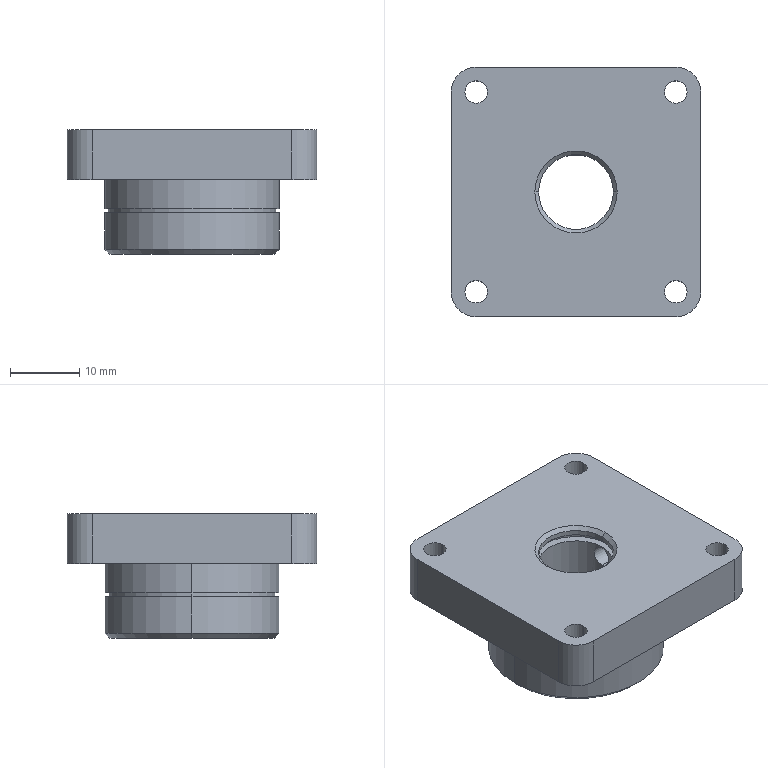Part | SolidWorks | features ICE 5, RevCut 3, Chamfer 2, Extrusion 1, Fillet 1 | 1 solid | 52 faces | box 36 x 36 x 18 mm | volume 12390 mm3 | cylinder 32 | plane 14 | cone 6 | commonest cylinder face diameters 3.24 x8 10.8 x6 7.2 x4 25.2 x4 3 x2 11.88 x2
STEP:
#1=CARTESIAN_POINT('',(5.4,0.,15.5));
#2=VERTEX_POINT('',#1);
#3=CARTESIAN_POINT('',(5.4,0.,12.5));
#4=VERTEX_POINT('',#3);
#5=CARTESIAN_POINT('',(5.4,0.,15.5));
#6=CARTESIAN_POINT('',(5.4,-0.1963,15.5));
#7=CARTESIAN_POINT('',(5.389,-0.3946,15.46));
#8=CARTESIAN_POINT('',(5.36,-0.6657,15.348));
#9=CARTESIAN_POINT('',(5.348,-0.7535,15.301));
#10=CARTESIAN_POINT('',(5.322,-0.916,15.192));
#11=CARTESIAN_POINT('',(5.309,-0.9912,15.13));
#12=CARTESIAN_POINT('',(5.281,-1.13,14.992));
#13=CARTESIAN_POINT('',(5.267,-1.192,14.915));
#14=CARTESIAN_POINT('',(5.241,-1.301,14.753));
#15=CARTESIAN_POINT('',(5.229,-1.347,14.667));
#16=CARTESIAN_POINT('',(5.199,-1.461,14.393));
#17=CARTESIAN_POINT('',(5.187,-1.5,14.198));
#18=CARTESIAN_POINT('',(5.187,-1.5,13.901));
#19=CARTESIAN_POINT('',(5.19,-1.49,13.804));
#20=CARTESIAN_POINT('',(5.201,-1.452,13.611));
#21=CARTESIAN_POINT('',(5.209,-1.423,13.515));
#22=CARTESIAN_POINT('',(5.239,-1.31,13.244));
#23=CARTESIAN_POINT('',(5.267,-1.199,13.077));
#24=CARTESIAN_POINT('',(5.322,-0.9237,12.802));
#25=CARTESIAN_POINT('',(5.35,-0.7576,12.691));
#26=CARTESIAN_POINT('',(5.379,-0.4865,12.578));
#27=CARTESIAN_POINT('',(5.387,-0.3908,12.548));
#28=CARTESIAN_POINT('',(5.397,-0.1977,12.51));
#29=CARTESIAN_POINT('',(5.4,-0.09961,12.5));
#30=CARTESIAN_POINT('',(5.4,0.,12.5));
#31=B_SPLINE_CURVE_WITH_KNOTS('',3,(#5,#6,#7,#8,#9,#10,#11,#12,#13,#14,#15,#16,#17,#18,#19,#20,#21,#22,#23,#24,#25,#26,#27,#28,#29,#30),.UNSPECIFIED.,.F.,.F.,(4,2,2,2,2,2,2,2,2,2,2,2,4),(0.004713,0.005302,0.005596,0.005891,0.006185,0.00648,0.007069,0.007363,0.007658,0.008247,0.008836,0.00913,0.009425),.UNSPECIFIED.);
#32=EDGE_CURVE('',#2,#4,#31,.T.);
#33=ORIENTED_EDGE('',*,*,#32,.F.);
#34=CARTESIAN_POINT('',(18.,0.,15.5));
#35=VERTEX_POINT('',#34);
#36=CARTESIAN_POINT('',(2.,0.,15.5));
#37=DIRECTION('',(1.,0.,0.));
#38=VECTOR('',#37,1000.);
#39=LINE('',#36,#38);
#40=EDGE_CURVE('',#2,#35,#39,.T.);
#41=ORIENTED_EDGE('',*,*,#40,.T.);
#42=CARTESIAN_POINT('',(18.,0.,12.5));
#43=VERTEX_POINT('',#42);
#44=CARTESIAN_POINT('',(18.,0.,14.));
#45=DIRECTION('',(1.,0.,0.));
#46=DIRECTION('',(0.,0.,-1.));
#47=AXIS2_PLACEMENT_3D('',#44,#45,#46);
#48=CIRCLE('',#47,1.5);
#49=EDGE_CURVE('',#35,#43,#48,.T.);
#50=ORIENTED_EDGE('',*,*,#49,.T.);
#51=CARTESIAN_POINT('',(2.,0.,12.5));
#52=DIRECTION('',(1.,0.,0.));
#53=VECTOR('',#52,1000.);
#54=LINE('',#51,#53);
#55=EDGE_CURVE('',#4,#43,#54,.T.);
#56=ORIENTED_EDGE('',*,*,#55,.F.);
#57=EDGE_LOOP('',(#33,#41,#50,#56));
#58=FACE_OUTER_BOUND('',#57,.T.);
#59=CARTESIAN_POINT('',(2.,0.,14.));
#60=DIRECTION('',(1.,0.,0.));
#61=DIRECTION('',(0.,0.,-1.));
#62=AXIS2_PLACEMENT_3D('',#59,#60,#61);
#63=CYLINDRICAL_SURFACE('',#62,1.5);
#64=ADVANCED_FACE('',(#58),#63,.F.);
#65=CARTESIAN_POINT('',(0.,6.48,15.66));
#66=VERTEX_POINT('',#65);
#67=CARTESIAN_POINT('',(0.,-6.48,15.66));
#68=VERTEX_POINT('',#67);
#69=CARTESIAN_POINT('',(0.,0.,15.66));
#70=DIRECTION('',(0.,0.,1.));
#71=DIRECTION('',(0.,-1.,0.));
#72=AXIS2_PLACEMENT_3D('',#69,#70,#71);
#73=CIRCLE('',#72,6.48);
#74=EDGE_CURVE('',#66,#68,#73,.T.);
#75=ORIENTED_EDGE('',*,*,#74,.F.);
#76=CARTESIAN_POINT('',(0.,6.48,16.74));
#77=VERTEX_POINT('',#76);
#78=CARTESIAN_POINT('',(0.,6.48,18.));
#79=DIRECTION('',(0.,0.,1.));
#80=VECTOR('',#79,1000.);
#81=LINE('',#78,#80);
#82=EDGE_CURVE('',#66,#77,#81,.T.);
#83=ORIENTED_EDGE('',*,*,#82,.T.);
#84=CARTESIAN_POINT('',(0.,-6.48,16.74));
#85=VERTEX_POINT('',#84);
#86=CARTESIAN_POINT('',(0.,0.,16.74));
#87=DIRECTION('',(0.,0.,1.));
#88=DIRECTION('',(0.,-1.,0.));
#89=AXIS2_PLACEMENT_3D('',#86,#87,#88);
#90=CIRCLE('',#89,6.48);
#91=EDGE_CURVE('',#77,#85,#90,.T.);
#92=ORIENTED_EDGE('',*,*,#91,.T.);
#93=CARTESIAN_POINT('',(0.,-6.48,18.));
#94=DIRECTION('',(0.,0.,1.));
#95=VECTOR('',#94,1000.);
#96=LINE('',#93,#95);
#97=EDGE_CURVE('',#68,#85,#96,.T.);
#98=ORIENTED_EDGE('',*,*,#97,.F.);
#99=EDGE_LOOP('',(#75,#83,#92,#98));
#100=FACE_OUTER_BOUND('',#99,.T.);
#101=CARTESIAN_POINT('',(0.,0.,18.));
#102=DIRECTION('',(0.,0.,1.));
#103=DIRECTION('',(0.,-1.,0.));
#104=AXIS2_PLACEMENT_3D('',#101,#102,#103);
#105=CYLINDRICAL_SURFACE('',#104,6.48);
#106=ADVANCED_FACE('',(#100),#105,.F.);
#107=CARTESIAN_POINT('',(0.,-5.94,3.87));
#108=VERTEX_POINT('',#107);
#109=CARTESIAN_POINT('',(0.,5.94,3.87));
#110=VERTEX_POINT('',#109);
#111=CARTESIAN_POINT('',(0.,0.,3.87));
#112=DIRECTION('',(0.,0.,-1.));
#113=DIRECTION('',(0.,1.,0.));
#114=AXIS2_PLACEMENT_3D('',#111,#112,#113);
#115=CIRCLE('',#114,5.94);
#116=EDGE_CURVE('',#108,#110,#115,.T.);
#117=ORIENTED_EDGE('',*,*,#116,.F.);
#118=CARTESIAN_POINT('',(0.,-5.94,3.33));
#119=VERTEX_POINT('',#118);
#120=CARTESIAN_POINT('',(0.,-5.94,0.));
#121=DIRECTION('',(0.,0.,-1.));
#122=VECTOR('',#121,1000.);
#123=LINE('',#120,#122);
#124=EDGE_CURVE('',#108,#119,#123,.T.);
#125=ORIENTED_EDGE('',*,*,#124,.T.);
#126=CARTESIAN_POINT('',(0.,5.94,3.33));
#127=VERTEX_POINT('',#126);
#128=CARTESIAN_POINT('',(0.,0.,3.33));
#129=DIRECTION('',(0.,0.,-1.));
#130=DIRECTION('',(0.,1.,0.));
#131=AXIS2_PLACEMENT_3D('',#128,#129,#130);
#132=CIRCLE('',#131,5.94);
#133=EDGE_CURVE('',#119,#127,#132,.T.);
#134=ORIENTED_EDGE('',*,*,#133,.T.);
#135=CARTESIAN_POINT('',(0.,5.94,0.));
#136=DIRECTION('',(0.,0.,-1.));
#137=VECTOR('',#136,1000.);
#138=LINE('',#135,#137);
#139=EDGE_CURVE('',#110,#127,#138,.T.);
#140=ORIENTED_EDGE('',*,*,#139,.F.);
#141=EDGE_LOOP('',(#117,#125,#134,#140));
#142=FACE_OUTER_BOUND('',#141,.T.);
#143=CARTESIAN_POINT('',(0.,0.,0.));
#144=DIRECTION('',(0.,0.,-1.));
#145=DIRECTION('',(0.,1.,0.));
#146=AXIS2_PLACEMENT_3D('',#143,#144,#145);
#147=CYLINDRICAL_SURFACE('',#146,5.94);
#148=ADVANCED_FACE('',(#142),#147,.F.);
#149=CARTESIAN_POINT('',(-12.06,0.,6.57));
#150=VERTEX_POINT('',#149);
#151=CARTESIAN_POINT('',(12.06,0.,6.57));
#152=VERTEX_POINT('',#151);
#153=CARTESIAN_POINT('',(0.,0.,6.57));
#154=DIRECTION('',(0.,0.,-1.));
#155=DIRECTION('',(-1.,0.,0.));
#156=AXIS2_PLACEMENT_3D('',#153,#154,#155);
#157=CIRCLE('',#156,12.06);
#158=EDGE_CURVE('',#150,#152,#157,.T.);
#159=ORIENTED_EDGE('',*,*,#158,.T.);
#160=CARTESIAN_POINT('',(12.06,0.,6.03));
#161=VERTEX_POINT('',#160);
#162=CARTESIAN_POINT('',(12.06,0.,0.));
#163=DIRECTION('',(0.,0.,-1.));
#164=VECTOR('',#163,1000.);
#165=LINE('',#162,#164);
#166=EDGE_CURVE('',#152,#161,#165,.T.);
#167=ORIENTED_EDGE('',*,*,#166,.T.);
#168=CARTESIAN_POINT('',(-12.06,0.,6.03));
#169=VERTEX_POINT('',#168);
#170=CARTESIAN_POINT('',(0.,0.,6.03));
#171=DIRECTION('',(0.,0.,-1.));
#172=DIRECTION('',(-1.,0.,0.));
#173=AXIS2_PLACEMENT_3D('',#170,#171,#172);
#174=CIRCLE('',#173,12.06);
#175=EDGE_CURVE('',#169,#161,#174,.T.);
#176=ORIENTED_EDGE('',*,*,#175,.F.);
#177=CARTESIAN_POINT('',(-12.06,0.,0.));
#178=DIRECTION('',(0.,0.,-1.));
#179=VECTOR('',#178,1000.);
#180=LINE('',#177,#179);
#181=EDGE_CURVE('',#150,#169,#180,.T.);
#182=ORIENTED_EDGE('',*,*,#181,.F.);
#183=EDGE_LOOP('',(#159,#167,#176,#182));
#184=FACE_OUTER_BOUND('',#183,.T.);
#185=CARTESIAN_POINT('',(0.,0.,0.));
#186=DIRECTION('',(0.,0.,-1.));
#187=DIRECTION('',(-1.,0.,0.));
#188=AXIS2_PLACEMENT_3D('',#185,#186,#187);
#189=CYLINDRICAL_SURFACE('',#188,12.06);
#190=ADVANCED_FACE('',(#184),#189,.T.);
#191=CARTESIAN_POINT('',(5.4,0.,0.54));
#192=VERTEX_POINT('',#191);
#193=CARTESIAN_POINT('',(-5.4,0.,0.54));
#194=VERTEX_POINT('',#193);
#195=CARTESIAN_POINT('',(0.,0.,0.54));
#196=DIRECTION('',(0.,0.,-1.));
#197=DIRECTION('',(1.,0.,0.));
#198=AXIS2_PLACEMENT_3D('',#195,#196,#197);
#199=CIRCLE('',#198,5.4);
#200=EDGE_CURVE('',#192,#194,#199,.T.);
#201=ORIENTED_EDGE('',*,*,#200,.F.);
#202=CARTESIAN_POINT('',(5.94,0.,0.));
#203=VERTEX_POINT('',#202);
#204=CARTESIAN_POINT('',(5.4,0.,0.54));
#205=DIRECTION('',(0.7071,0.,-0.7071));
#206=VECTOR('',#205,1000.);
#207=LINE('',#204,#206);
#208=EDGE_CURVE('',#192,#203,#207,.T.);
#209=ORIENTED_EDGE('',*,*,#208,.T.);
#210=CARTESIAN_POINT('',(-5.94,0.,0.));
#211=VERTEX_POINT('',#210);
#212=CARTESIAN_POINT('',(0.,0.,0.));
#213=DIRECTION('',(0.,0.,1.));
#214=DIRECTION('',(1.,0.,0.));
#215=AXIS2_PLACEMENT_3D('',#212,#213,#214);
#216=CIRCLE('',#215,5.94);
#217=EDGE_CURVE('',#211,#203,#216,.T.);
#218=ORIENTED_EDGE('',*,*,#217,.F.);
#219=CARTESIAN_POINT('',(-5.4,0.,0.54));
#220=DIRECTION('',(-0.7071,0.,-0.7071));
#221=VECTOR('',#220,1000.);
#222=LINE('',#219,#221);
#223=EDGE_CURVE('',#194,#211,#222,.T.);
#224=ORIENTED_EDGE('',*,*,#223,.F.);
#225=EDGE_LOOP('',(#201,#209,#218,#224));
#226=FACE_OUTER_BOUND('',#225,.T.);
#227=CARTESIAN_POINT('',(0.,0.,0.54));
#228=DIRECTION('',(0.,0.,-1.));
#229=DIRECTION('',(-1.,0.,0.));
#230=AXIS2_PLACEMENT_3D('',#227,#228,#229);
#231=CONICAL_SURFACE('',#230,5.4,0.7854);
#232=ADVANCED_FACE('',(#226),#231,.F.);
#233=CARTESIAN_POINT('',(-5.4,0.,17.46));
#234=VERTEX_POINT('',#233);
#235=CARTESIAN_POINT('',(5.4,0.,17.46));
#236=VERTEX_POINT('',#235);
#237=CARTESIAN_POINT('',(0.,0.,17.46));
#238=DIRECTION('',(0.,0.,1.));
#239=DIRECTION('',(-1.,0.,0.));
#240=AXIS2_PLACEMENT_3D('',#237,#238,#239);
#241=CIRCLE('',#240,5.4);
#242=EDGE_CURVE('',#234,#236,#241,.T.);
#243=ORIENTED_EDGE('',*,*,#242,.F.);
#244=CARTESIAN_POINT('',(-5.94,0.,18.));
#245=VERTEX_POINT('',#244);
#246=CARTESIAN_POINT('',(-5.94,0.,18.));
#247=DIRECTION('',(-0.7071,0.,0.7071));
#248=VECTOR('',#247,1000.);
#249=LINE('',#246,#248);
#250=EDGE_CURVE('',#234,#245,#249,.T.);
#251=ORIENTED_EDGE('',*,*,#250,.T.);
#252=CARTESIAN_POINT('',(5.94,0.,18.));
#253=VERTEX_POINT('',#252);
#254=CARTESIAN_POINT('',(0.,0.,18.));
#255=DIRECTION('',(0.,0.,-1.));
#256=DIRECTION('',(-1.,0.,0.));
#257=AXIS2_PLACEMENT_3D('',#254,#255,#256);
#258=CIRCLE('',#257,5.94);
#259=EDGE_CURVE('',#253,#245,#258,.T.);
#260=ORIENTED_EDGE('',*,*,#259,.F.);
#261=CARTESIAN_POINT('',(5.94,0.,18.));
#262=DIRECTION('',(0.7071,0.,0.7071));
#263=VECTOR('',#262,1000.);
#264=LINE('',#261,#263);
#265=EDGE_CURVE('',#236,#253,#264,.T.);
#266=ORIENTED_EDGE('',*,*,#265,.F.);
#267=EDGE_LOOP('',(#243,#251,#260,#266));
#268=FACE_OUTER_BOUND('',#267,.T.);
#269=CARTESIAN_POINT('',(0.,0.,18.));
#270=DIRECTION('',(0.,0.,1.));
#271=DIRECTION('',(1.,0.,0.));
#272=AXIS2_PLACEMENT_3D('',#269,#270,#271);
#273=CONICAL_SURFACE('',#272,5.94,0.7854);
#274=ADVANCED_FACE('',(#268),#273,.F.);
#275=CARTESIAN_POINT('',(-12.78,14.4,18.));
#276=VERTEX_POINT('',#275);
#277=CARTESIAN_POINT('',(-16.02,14.4,18.));
#278=VERTEX_POINT('',#277);
#279=CARTESIAN_POINT('',(-14.4,14.4,18.));
#280=DIRECTION('',(0.,0.,-1.));
#281=DIRECTION('',(-1.,0.,0.));
#282=AXIS2_PLACEMENT_3D('',#279,#280,#281);
#283=CIRCLE('',#282,1.62);
#284=EDGE_CURVE('',#276,#278,#283,.T.);
#285=ORIENTED_EDGE('',*,*,#284,.F.);
#286=CARTESIAN_POINT('',(-12.78,14.4,10.8));
#287=VERTEX_POINT('',#286);
#288=CARTESIAN_POINT('',(-12.78,14.4,18.));
#289=DIRECTION('',(0.,0.,-1.));
#290=VECTOR('',#289,1000.);
#291=LINE('',#288,#290);
#292=EDGE_CURVE('',#276,#287,#291,.T.);
#293=ORIENTED_EDGE('',*,*,#292,.T.);
#294=CARTESIAN_POINT('',(-16.02,14.4,10.8));
#295=VERTEX_POINT('',#294);
#296=CARTESIAN_POINT('',(-14.4,14.4,10.8));
#297=DIRECTION('',(0.,0.,-1.));
#298=DIRECTION('',(-1.,0.,0.));
#299=AXIS2_PLACEMENT_3D('',#296,#297,#298);
#300=CIRCLE('',#299,1.62);
#301=EDGE_CURVE('',#287,#295,#300,.T.);
#302=ORIENTED_EDGE('',*,*,#301,.T.);
#303=CARTESIAN_POINT('',(-16.02,14.4,18.));
#304=DIRECTION('',(0.,0.,-1.));
#305=VECTOR('',#304,1000.);
#306=LINE('',#303,#305);
#307=EDGE_CURVE('',#278,#295,#306,.T.);
#308=ORIENTED_EDGE('',*,*,#307,.F.);
#309=EDGE_LOOP('',(#285,#293,#302,#308));
#310=FACE_OUTER_BOUND('',#309,.T.);
#311=CARTESIAN_POINT('',(-14.4,14.4,18.));
#312=DIRECTION('',(0.,0.,-1.));
#313=DIRECTION('',(-1.,0.,0.));
#314=AXIS2_PLACEMENT_3D('',#311,#312,#313);
#315=CYLINDRICAL_SURFACE('',#314,1.62);
#316=ADVANCED_FACE('',(#310),#315,.F.);
#317=CARTESIAN_POINT('',(-12.78,-14.4,18.));
#318=VERTEX_POINT('',#317);
#319=CARTESIAN_POINT('',(-16.02,-14.4,18.));
#320=VERTEX_POINT('',#319);
#321=CARTESIAN_POINT('',(-14.4,-14.4,18.));
#322=DIRECTION('',(0.,0.,-1.));
#323=DIRECTION('',(-1.,0.,0.));
#324=AXIS2_PLACEMENT_3D('',#321,#322,#323);
#325=CIRCLE('',#324,1.62);
#326=EDGE_CURVE('',#318,#320,#325,.T.);
#327=ORIENTED_EDGE('',*,*,#326,.F.);
#328=CARTESIAN_POINT('',(-12.78,-14.4,10.8));
#329=VERTEX_POINT('',#328);
#330=CARTESIAN_POINT('',(-12.78,-14.4,18.));
#331=DIRECTION('',(0.,0.,-1.));
#332=VECTOR('',#331,1000.);
#333=LINE('',#330,#332);
#334=EDGE_CURVE('',#318,#329,#333,.T.);
#335=ORIENTED_EDGE('',*,*,#334,.T.);
#336=CARTESIAN_POINT('',(-16.02,-14.4,10.8));
#337=VERTEX_POINT('',#336);
#338=CARTESIAN_POINT('',(-14.4,-14.4,10.8));
#339=DIRECTION('',(0.,0.,-1.));
#340=DIRECTION('',(-1.,0.,0.));
#341=AXIS2_PLACEMENT_3D('',#338,#339,#340);
#342=CIRCLE('',#341,1.62);
#343=EDGE_CURVE('',#329,#337,#342,.T.);
#344=ORIENTED_EDGE('',*,*,#343,.T.);
#345=CARTESIAN_POINT('',(-16.02,-14.4,18.));
#346=DIRECTION('',(0.,0.,-1.));
#347=VECTOR('',#346,1000.);
#348=LINE('',#345,#347);
#349=EDGE_CURVE('',#320,#337,#348,.T.);
#350=ORIENTED_EDGE('',*,*,#349,.F.);
#351=EDGE_LOOP('',(#327,#335,#344,#350));
#352=FACE_OUTER_BOUND('',#351,.T.);
#353=CARTESIAN_POINT('',(-14.4,-14.4,18.));
#354=DIRECTION('',(0.,0.,-1.));
#355=DIRECTION('',(-1.,0.,0.));
#356=AXIS2_PLACEMENT_3D('',#353,#354,#355);
#357=CYLINDRICAL_SURFACE('',#356,1.62);
#358=ADVANCED_FACE('',(#352),#357,.F.);
#359=CARTESIAN_POINT('',(16.02,-14.4,18.));
#360=VERTEX_POINT('',#359);
#361=CARTESIAN_POINT('',(12.78,-14.4,18.));
#362=VERTEX_POINT('',#361);
#363=CARTESIAN_POINT('',(14.4,-14.4,18.));
#364=DIRECTION('',(0.,0.,-1.));
#365=DIRECTION('',(-1.,0.,0.));
#366=AXIS2_PLACEMENT_3D('',#363,#364,#365);
#367=CIRCLE('',#366,1.62);
#368=EDGE_CURVE('',#360,#362,#367,.T.);
#369=ORIENTED_EDGE('',*,*,#368,.F.);
#370=CARTESIAN_POINT('',(16.02,-14.4,10.8));
#371=VERTEX_POINT('',#370);
#372=CARTESIAN_POINT('',(16.02,-14.4,18.));
#373=DIRECTION('',(0.,0.,-1.));
#374=VECTOR('',#373,1000.);
#375=LINE('',#372,#374);
#376=EDGE_CURVE('',#360,#371,#375,.T.);
#377=ORIENTED_EDGE('',*,*,#376,.T.);
#378=CARTESIAN_POINT('',(12.78,-14.4,10.8));
#379=VERTEX_POINT('',#378);
#380=CARTESIAN_POINT('',(14.4,-14.4,10.8));
#381=DIRECTION('',(0.,0.,-1.));
#382=DIRECTION('',(-1.,0.,0.));
#383=AXIS2_PLACEMENT_3D('',#380,#381,#382);
#384=CIRCLE('',#383,1.62);
#385=EDGE_CURVE('',#371,#379,#384,.T.);
#386=ORIENTED_EDGE('',*,*,#385,.T.);
#387=CARTESIAN_POINT('',(12.78,-14.4,18.));
#388=DIRECTION('',(0.,0.,-1.));
#389=VECTOR('',#388,1000.);
#390=LINE('',#387,#389);
#391=EDGE_CURVE('',#362,#379,#390,.T.);
#392=ORIENTED_EDGE('',*,*,#391,.F.);
#393=EDGE_LOOP('',(#369,#377,#386,#392));
#394=FACE_OUTER_BOUND('',#393,.T.);
#395=CARTESIAN_POINT('',(14.4,-14.4,18.));
#396=DIRECTION('',(0.,0.,-1.));
#397=DIRECTION('',(-1.,0.,0.));
#398=AXIS2_PLACEMENT_3D('',#395,#396,#397);
#399=CYLINDRICAL_SURFACE('',#398,1.62);
#400=ADVANCED_FACE('',(#394),#399,.F.);
#401=CARTESIAN_POINT('',(16.02,14.4,18.));
#402=VERTEX_POINT('',#401);
#403=CARTESIAN_POINT('',(12.78,14.4,18.));
#404=VERTEX_POINT('',#403);
#405=CARTESIAN_POINT('',(14.4,14.4,18.));
#406=DIRECTION('',(0.,0.,-1.));
#407=DIRECTION('',(-1.,0.,0.));
#408=AXIS2_PLACEMENT_3D('',#405,#406,#407);
#409=CIRCLE('',#408,1.62);
#410=EDGE_CURVE('',#402,#404,#409,.T.);
#411=ORIENTED_EDGE('',*,*,#410,.F.);
#412=CARTESIAN_POINT('',(16.02,14.4,10.8));
#413=VERTEX_POINT('',#412);
#414=CARTESIAN_POINT('',(16.02,14.4,18.));
#415=DIRECTION('',(0.,0.,-1.));
#416=VECTOR('',#415,1000.);
#417=LINE('',#414,#416);
#418=EDGE_CURVE('',#402,#413,#417,.T.);
#419=ORIENTED_EDGE('',*,*,#418,.T.);
#420=CARTESIAN_POINT('',(12.78,14.4,10.8));
#421=VERTEX_POINT('',#420);
#422=CARTESIAN_POINT('',(14.4,14.4,10.8));
#423=DIRECTION('',(0.,0.,-1.));
#424=DIRECTION('',(-1.,0.,0.));
#425=AXIS2_PLACEMENT_3D('',#422,#423,#424);
#426=CIRCLE('',#425,1.62);
#427=EDGE_CURVE('',#413,#421,#426,.T.);
#428=ORIENTED_EDGE('',*,*,#427,.T.);
#429=CARTESIAN_POINT('',(12.78,14.4,18.));
#430=DIRECTION('',(0.,0.,-1.));
#431=VECTOR('',#430,1000.);
#432=LINE('',#429,#431);
#433=EDGE_CURVE('',#404,#421,#432,.T.);
#434=ORIENTED_EDGE('',*,*,#433,.F.);
#435=EDGE_LOOP('',(#411,#419,#428,#434));
#436=FACE_OUTER_BOUND('',#435,.T.);
#437=CARTESIAN_POINT('',(14.4,14.4,18.));
#438=DIRECTION('',(0.,0.,-1.));
#439=DIRECTION('',(-1.,0.,0.));
#440=AXIS2_PLACEMENT_3D('',#437,#438,#439);
#441=CYLINDRICAL_SURFACE('',#440,1.62);
#442=ADVANCED_FACE('',(#436),#441,.F.);
#443=CARTESIAN_POINT('',(-12.6,0.,6.03));
#444=VERTEX_POINT('',#443);
#445=CARTESIAN_POINT('',(12.6,0.,6.03));
#446=VERTEX_POINT('',#445);
#447=CARTESIAN_POINT('',(0.,0.,6.03));
#448=DIRECTION('',(0.,0.,-1.));
#449=DIRECTION('',(-1.,0.,0.));
#450=AXIS2_PLACEMENT_3D('',#447,#448,#449);
#451=CIRCLE('',#450,12.6);
#452=EDGE_CURVE('',#444,#446,#451,.T.);
#453=ORIENTED_EDGE('',*,*,#452,.T.);
#454=CARTESIAN_POINT('',(12.6,0.,0.72));
#455=VERTEX_POINT('',#454);
#456=CARTESIAN_POINT('',(12.6,0.,10.8));
#457=DIRECTION('',(0.,0.,-1.));
#458=VECTOR('',#457,1000.);
#459=LINE('',#456,#458);
#460=EDGE_CURVE('',#446,#455,#459,.T.);
#461=ORIENTED_EDGE('',*,*,#460,.T.);
#462=CARTESIAN_POINT('',(-12.6,0.,0.72));
#463=VERTEX_POINT('',#462);
#464=CARTESIAN_POINT('',(0.,0.,0.72));
#465=DIRECTION('',(0.,0.,1.));
#466=DIRECTION('',(1.,0.,0.));
#467=AXIS2_PLACEMENT_3D('',#464,#465,#466);
#468=CIRCLE('',#467,12.6);
#469=EDGE_CURVE('',#455,#463,#468,.T.);
#470=ORIENTED_EDGE('',*,*,#469,.T.);
#471=CARTESIAN_POINT('',(-12.6,0.,10.8));
#472=DIRECTION('',(0.,0.,-1.));
#473=VECTOR('',#472,1000.);
#474=LINE('',#471,#473);
#475=EDGE_CURVE('',#444,#463,#474,.T.);
#476=ORIENTED_EDGE('',*,*,#475,.F.);
#477=EDGE_LOOP('',(#453,#461,#470,#476));
#478=FACE_OUTER_BOUND('',#477,.T.);
#479=CARTESIAN_POINT('',(0.,0.,10.8));
#480=DIRECTION('',(0.,0.,-1.));
#481=DIRECTION('',(-1.,0.,0.));
#482=AXIS2_PLACEMENT_3D('',#479,#480,#481);
#483=CYLINDRICAL_SURFACE('',#482,12.6);
#484=ADVANCED_FACE('',(#478),#483,.T.);
#485=CARTESIAN_POINT('',(-11.88,0.,0.));
#486=VERTEX_POINT('',#485);
#487=CARTESIAN_POINT('',(11.88,0.,0.));
#488=VERTEX_POINT('',#487);
#489=CARTESIAN_POINT('',(0.,0.,0.));
#490=DIRECTION('',(0.,0.,-1.));
#491=DIRECTION('',(1.,0.,0.));
#492=AXIS2_PLACEMENT_3D('',#489,#490,#491);
#493=CIRCLE('',#492,11.88);
#494=EDGE_CURVE('',#486,#488,#493,.T.);
#495=ORIENTED_EDGE('',*,*,#494,.F.);
#496=CARTESIAN_POINT('',(-12.6,0.,0.72));
#497=DIRECTION('',(-0.7071,0.,0.7071));
#498=VECTOR('',#497,1000.);
#499=LINE('',#496,#498);
#500=EDGE_CURVE('',#486,#463,#499,.T.);
#501=ORIENTED_EDGE('',*,*,#500,.T.);
#502=ORIENTED_EDGE('',*,*,#469,.F.);
#503=CARTESIAN_POINT('',(12.6,0.,0.72));
#504=DIRECTION('',(0.7071,0.,0.7071));
#505=VECTOR('',#504,1000.);
#506=LINE('',#503,#505);
#507=EDGE_CURVE('',#488,#455,#506,.T.);
#508=ORIENTED_EDGE('',*,*,#507,.F.);
#509=EDGE_LOOP('',(#495,#501,#502,#508));
#510=FACE_OUTER_BOUND('',#509,.T.);
#511=CARTESIAN_POINT('',(0.,0.,0.72));
#512=DIRECTION('',(0.,0.,1.));
#513=DIRECTION('',(1.,0.,0.));
#514=AXIS2_PLACEMENT_3D('',#511,#512,#513);
#515=CONICAL_SURFACE('',#514,12.6,0.7854);
#516=ADVANCED_FACE('',(#510),#515,.T.);
#517=CARTESIAN_POINT('',(14.4,0.,11.88));
#518=VERTEX_POINT('',#517);
#519=CARTESIAN_POINT('',(-14.4,0.,11.88));
#520=VERTEX_POINT('',#519);
#521=CARTESIAN_POINT('',(0.,0.,11.88));
#522=DIRECTION('',(0.,0.,-1.));
#523=DIRECTION('',(-1.,0.,0.));
#524=AXIS2_PLACEMENT_3D('',#521,#522,#523);
#525=CIRCLE('',#524,14.4);
#526=EDGE_CURVE('',#518,#520,#525,.T.);
#527=ORIENTED_EDGE('',*,*,#526,.F.);
#528=CARTESIAN_POINT('',(14.4,0.,10.8));
#529=VERTEX_POINT('',#528);
#530=CARTESIAN_POINT('',(14.4,0.,11.88));
#531=DIRECTION('',(0.,0.,-1.));
#532=VECTOR('',#531,1000.);
#533=LINE('',#530,#532);
#534=EDGE_CURVE('',#518,#529,#533,.T.);
#535=ORIENTED_EDGE('',*,*,#534,.T.);
#536=CARTESIAN_POINT('',(-14.4,0.,10.8));
#537=VERTEX_POINT('',#536);
#538=CARTESIAN_POINT('',(0.,0.,10.8));
#539=DIRECTION('',(0.,0.,-1.));
#540=DIRECTION('',(-1.,0.,0.));
#541=AXIS2_PLACEMENT_3D('',#538,#539,#540);
#542=CIRCLE('',#541,14.4);
#543=EDGE_CURVE('',#529,#537,#542,.T.);
#544=ORIENTED_EDGE('',*,*,#543,.T.);
#545=CARTESIAN_POINT('',(-14.4,0.,11.88));
#546=DIRECTION('',(0.,0.,-1.));
#547=VECTOR('',#546,1000.);
#548=LINE('',#545,#547);
#549=EDGE_CURVE('',#520,#537,#548,.T.);
#550=ORIENTED_EDGE('',*,*,#549,.F.);
#551=EDGE_LOOP('',(#527,#535,#544,#550));
#552=FACE_OUTER_BOUND('',#551,.T.);
#553=CARTESIAN_POINT('',(0.,0.,11.88));
#554=DIRECTION('',(0.,0.,-1.));
#555=DIRECTION('',(-1.,0.,0.));
#556=AXIS2_PLACEMENT_3D('',#553,#554,#555);
#557=CYLINDRICAL_SURFACE('',#556,14.4);
#558=ADVANCED_FACE('',(#552),#557,.F.);
#559=CARTESIAN_POINT('',(-12.6,0.,11.88));
#560=VERTEX_POINT('',#559);
#561=CARTESIAN_POINT('',(12.6,0.,11.88));
#562=VERTEX_POINT('',#561);
#563=CARTESIAN_POINT('',(0.,0.,11.88));
#564=DIRECTION('',(0.,0.,-1.));
#565=DIRECTION('',(-1.,0.,0.));
#566=AXIS2_PLACEMENT_3D('',#563,#564,#565);
#567=CIRCLE('',#566,12.6);
#568=EDGE_CURVE('',#560,#562,#567,.T.);
#569=ORIENTED_EDGE('',*,*,#568,.T.);
#570=CARTESIAN_POINT('',(12.6,0.,6.57));
#571=VERTEX_POINT('',#570);
#572=CARTESIAN_POINT('',(12.6,0.,10.8));
#573=DIRECTION('',(0.,0.,-1.));
#574=VECTOR('',#573,1000.);
#575=LINE('',#572,#574);
#576=EDGE_CURVE('',#562,#571,#575,.T.);
#577=ORIENTED_EDGE('',*,*,#576,.T.);
#578=CARTESIAN_POINT('',(-12.6,0.,6.57));
#579=VERTEX_POINT('',#578);
#580=CARTESIAN_POINT('',(0.,0.,6.57));
#581=DIRECTION('',(0.,0.,-1.));
#582=DIRECTION('',(-1.,0.,0.));
#583=AXIS2_PLACEMENT_3D('',#580,#581,#582);
#584=CIRCLE('',#583,12.6);
#585=EDGE_CURVE('',#579,#571,#584,.T.);
#586=ORIENTED_EDGE('',*,*,#585,.F.);
#587=CARTESIAN_POINT('',(-12.6,0.,10.8));
#588=DIRECTION('',(0.,0.,-1.));
#589=VECTOR('',#588,1000.);
#590=LINE('',#587,#589);
#591=EDGE_CURVE('',#560,#579,#590,.T.);
#592=ORIENTED_EDGE('',*,*,#591,.F.);
#593=EDGE_LOOP('',(#569,#577,#586,#592));
#594=FACE_OUTER_BOUND('',#593,.T.);
#595=CARTESIAN_POINT('',(0.,0.,10.8));
#596=DIRECTION('',(0.,0.,-1.));
#597=DIRECTION('',(-1.,0.,0.));
#598=AXIS2_PLACEMENT_3D('',#595,#596,#597);
#599=CYLINDRICAL_SURFACE('',#598,12.6);
#600=ADVANCED_FACE('',(#594),#599,.T.);
#601=CARTESIAN_POINT('',(-5.4,0.,3.33));
#602=VERTEX_POINT('',#601);
#603=CARTESIAN_POINT('',(5.4,0.,3.33));
#604=VERTEX_POINT('',#603);
#605=CARTESIAN_POINT('',(0.,0.,3.33));
#606=DIRECTION('',(0.,0.,1.));
#607=DIRECTION('',(0.,1.,0.));
#608=AXIS2_PLACEMENT_3D('',#605,#606,#607);
#609=CIRCLE('',#608,5.4);
#610=EDGE_CURVE('',#602,#604,#609,.T.);
#611=ORIENTED_EDGE('',*,*,#610,.T.);
#612=CARTESIAN_POINT('',(5.4,0.,18.));
#613=DIRECTION('',(0.,0.,-1.));
#614=VECTOR('',#613,1000.);
#615=LINE('',#612,#614);
#616=EDGE_CURVE('',#604,#192,#615,.T.);
#617=ORIENTED_EDGE('',*,*,#616,.T.);
#618=ORIENTED_EDGE('',*,*,#200,.T.);
#619=CARTESIAN_POINT('',(-5.4,0.,18.));
#620=DIRECTION('',(0.,0.,-1.));
#621=VECTOR('',#620,1000.);
#622=LINE('',#619,#621);
#623=EDGE_CURVE('',#602,#194,#622,.T.);
#624=ORIENTED_EDGE('',*,*,#623,.F.);
#625=EDGE_LOOP('',(#611,#617,#618,#624));
#626=FACE_OUTER_BOUND('',#625,.T.);
#627=CARTESIAN_POINT('',(0.,0.,18.));
#628=DIRECTION('',(0.,0.,-1.));
#629=DIRECTION('',(-1.,0.,0.));
#630=AXIS2_PLACEMENT_3D('',#627,#628,#629);
#631=CYLINDRICAL_SURFACE('',#630,5.4);
#632=ADVANCED_FACE('',(#626),#631,.F.);
#633=ORIENTED_EDGE('',*,*,#242,.T.);
#634=CARTESIAN_POINT('',(5.4,0.,16.74));
#635=VERTEX_POINT('',#634);
#636=CARTESIAN_POINT('',(5.4,0.,18.));
#637=DIRECTION('',(0.,0.,-1.));
#638=VECTOR('',#637,1000.);
#639=LINE('',#636,#638);
#640=EDGE_CURVE('',#236,#635,#639,.T.);
#641=ORIENTED_EDGE('',*,*,#640,.T.);
#642=CARTESIAN_POINT('',(-5.4,0.,16.74));
#643=VERTEX_POINT('',#642);
#644=CARTESIAN_POINT('',(0.,0.,16.74));
#645=DIRECTION('',(0.,0.,1.));
#646=DIRECTION('',(0.,1.,0.));
#647=AXIS2_PLACEMENT_3D('',#644,#645,#646);
#648=CIRCLE('',#647,5.4);
#649=EDGE_CURVE('',#643,#635,#648,.T.);
#650=ORIENTED_EDGE('',*,*,#649,.F.);
#651=CARTESIAN_POINT('',(-5.4,0.,18.));
#652=DIRECTION('',(0.,0.,-1.));
#653=VECTOR('',#652,1000.);
#654=LINE('',#651,#653);
#655=EDGE_CURVE('',#234,#643,#654,.T.);
#656=ORIENTED_EDGE('',*,*,#655,.F.);
#657=EDGE_LOOP('',(#633,#641,#650,#656));
#658=FACE_OUTER_BOUND('',#657,.T.);
#659=CARTESIAN_POINT('',(0.,0.,18.));
#660=DIRECTION('',(0.,0.,-1.));
#661=DIRECTION('',(-1.,0.,0.));
#662=AXIS2_PLACEMENT_3D('',#659,#660,#661);
#663=CYLINDRICAL_SURFACE('',#662,5.4);
#664=ADVANCED_FACE('',(#658),#663,.F.);
#665=CARTESIAN_POINT('',(5.4,0.,15.66));
#666=VERTEX_POINT('',#665);
#667=CARTESIAN_POINT('',(-5.4,0.,15.66));
#668=VERTEX_POINT('',#667);
#669=CARTESIAN_POINT('',(0.,0.,15.66));
#670=DIRECTION('',(0.,0.,-1.));
#671=DIRECTION('',(0.,-1.,0.));
#672=AXIS2_PLACEMENT_3D('',#669,#670,#671);
#673=CIRCLE('',#672,5.4);
#674=EDGE_CURVE('',#666,#668,#673,.T.);
#675=ORIENTED_EDGE('',*,*,#674,.F.);
#676=CARTESIAN_POINT('',(5.4,0.,18.));
#677=DIRECTION('',(0.,0.,-1.));
#678=VECTOR('',#677,1000.);
#679=LINE('',#676,#678);
#680=EDGE_CURVE('',#666,#2,#679,.T.);
#681=ORIENTED_EDGE('',*,*,#680,.T.);
#682=ORIENTED_EDGE('',*,*,#32,.T.);
#683=CARTESIAN_POINT('',(5.4,0.,3.87));
#684=VERTEX_POINT('',#683);
#685=CARTESIAN_POINT('',(5.4,0.,18.));
#686=DIRECTION('',(0.,0.,-1.));
#687=VECTOR('',#686,1000.);
#688=LINE('',#685,#687);
#689=EDGE_CURVE('',#4,#684,#688,.T.);
#690=ORIENTED_EDGE('',*,*,#689,.T.);
#691=CARTESIAN_POINT('',(-5.4,0.,3.87));
#692=VERTEX_POINT('',#691);
#693=CARTESIAN_POINT('',(0.,0.,3.87));
#694=DIRECTION('',(0.,0.,-1.));
#695=DIRECTION('',(0.,-1.,0.));
#696=AXIS2_PLACEMENT_3D('',#693,#694,#695);
#697=CIRCLE('',#696,5.4);
#698=EDGE_CURVE('',#684,#692,#697,.T.);
#699=ORIENTED_EDGE('',*,*,#698,.T.);
#700=CARTESIAN_POINT('',(-5.4,0.,18.));
#701=DIRECTION('',(0.,0.,-1.));
#702=VECTOR('',#701,1000.);
#703=LINE('',#700,#702);
#704=EDGE_CURVE('',#668,#692,#703,.T.);
#705=ORIENTED_EDGE('',*,*,#704,.F.);
#706=EDGE_LOOP('',(#675,#681,#682,#690,#699,#705));
#707=FACE_OUTER_BOUND('',#706,.T.);
#708=CARTESIAN_POINT('',(0.,0.,18.));
#709=DIRECTION('',(0.,0.,-1.));
#710=DIRECTION('',(-1.,0.,0.));
#711=AXIS2_PLACEMENT_3D('',#708,#709,#710);
#712=CYLINDRICAL_SURFACE('',#711,5.4);
#713=ADVANCED_FACE('',(#707),#712,.F.);
#714=ORIENTED_EDGE('',*,*,#680,.F.);
#715=CARTESIAN_POINT('',(0.,0.,15.66));
#716=DIRECTION('',(0.,0.,-1.));
#717=DIRECTION('',(0.,-1.,0.));
#718=AXIS2_PLACEMENT_3D('',#715,#716,#717);
#719=CIRCLE('',#718,5.4);
#720=EDGE_CURVE('',#668,#666,#719,.T.);
#721=ORIENTED_EDGE('',*,*,#720,.F.);
#722=ORIENTED_EDGE('',*,*,#704,.T.);
#723=CARTESIAN_POINT('',(0.,0.,3.87));
#724=DIRECTION('',(0.,0.,-1.));
#725=DIRECTION('',(0.,-1.,0.));
#726=AXIS2_PLACEMENT_3D('',#723,#724,#725);
#727=CIRCLE('',#726,5.4);
#728=EDGE_CURVE('',#692,#684,#727,.T.);
#729=ORIENTED_EDGE('',*,*,#728,.T.);
#730=ORIENTED_EDGE('',*,*,#689,.F.);
#731=CARTESIAN_POINT('',(5.4,0.,12.5));
#732=CARTESIAN_POINT('',(5.4,0.09964,12.5));
#733=CARTESIAN_POINT('',(5.397,0.1975,12.51));
#734=CARTESIAN_POINT('',(5.387,0.3899,12.548));
#735=CARTESIAN_POINT('',(5.379,0.4855,12.577));
#736=CARTESIAN_POINT('',(5.359,0.6669,12.653));
#737=CARTESIAN_POINT('',(5.348,0.7529,12.699));
#738=CARTESIAN_POINT('',(5.322,0.9156,12.808));
#739=CARTESIAN_POINT('',(5.309,0.9922,12.871));
#740=CARTESIAN_POINT('',(5.267,1.199,13.077));
#741=CARTESIAN_POINT('',(5.239,1.31,13.244));
#742=CARTESIAN_POINT('',(5.199,1.46,13.605));
#743=CARTESIAN_POINT('',(5.188,1.5,13.803));
#744=CARTESIAN_POINT('',(5.187,1.5,14.098));
#745=CARTESIAN_POINT('',(5.19,1.49,14.198));
#746=CARTESIAN_POINT('',(5.201,1.452,14.39));
#747=CARTESIAN_POINT('',(5.209,1.423,14.484));
#748=CARTESIAN_POINT('',(5.239,1.31,14.758));
#749=CARTESIAN_POINT('',(5.267,1.199,14.922));
#750=CARTESIAN_POINT('',(5.309,0.991,15.13));
#751=CARTESIAN_POINT('',(5.322,0.9158,15.192));
#752=CARTESIAN_POINT('',(5.348,0.7537,15.301));
#753=CARTESIAN_POINT('',(5.36,0.6658,15.348));
#754=CARTESIAN_POINT('',(5.379,0.4848,15.423));
#755=CARTESIAN_POINT('',(5.387,0.3913,15.451));
#756=CARTESIAN_POINT('',(5.397,0.1978,15.49));
#757=CARTESIAN_POINT('',(5.4,0.0982,15.5));
#758=CARTESIAN_POINT('',(5.4,0.,15.5));
#759=B_SPLINE_CURVE_WITH_KNOTS('',3,(#731,#732,#733,#734,#735,#736,#737,#738,#739,#740,#741,#742,#743,#744,#745,#746,#747,#748,#749,#750,#751,#752,#753,#754,#755,#756,#757,#758),.UNSPECIFIED.,.F.,.F.,(4,2,2,2,2,2,2,2,2,2,2,2,2,4),(0.,0.0002946,0.0005891,0.0008837,0.001178,0.001767,0.002356,0.002651,0.002946,0.003535,0.003829,0.004124,0.004418,0.004713),.UNSPECIFIED.);
#760=EDGE_CURVE('',#4,#2,#759,.T.);
#761=ORIENTED_EDGE('',*,*,#760,.T.);
#762=EDGE_LOOP('',(#714,#721,#722,#729,#730,#761));
#763=FACE_OUTER_BOUND('',#762,.T.);
#764=CARTESIAN_POINT('',(0.,0.,18.));
#765=DIRECTION('',(0.,0.,-1.));
#766=DIRECTION('',(-1.,0.,0.));
#767=AXIS2_PLACEMENT_3D('',#764,#765,#766);
#768=CYLINDRICAL_SURFACE('',#767,5.4);
#769=ADVANCED_FACE('',(#763),#768,.F.);
#770=ORIENTED_EDGE('',*,*,#640,.F.);
#771=CARTESIAN_POINT('',(0.,0.,17.46));
#772=DIRECTION('',(0.,0.,1.));
#773=DIRECTION('',(-1.,0.,0.));
#774=AXIS2_PLACEMENT_3D('',#771,#772,#773);
#775=CIRCLE('',#774,5.4);
#776=EDGE_CURVE('',#236,#234,#775,.T.);
#777=ORIENTED_EDGE('',*,*,#776,.T.);
#778=ORIENTED_EDGE('',*,*,#655,.T.);
#779=CARTESIAN_POINT('',(0.,0.,16.74));
#780=DIRECTION('',(0.,0.,1.));
#781=DIRECTION('',(0.,1.,0.));
#782=AXIS2_PLACEMENT_3D('',#779,#780,#781);
#783=CIRCLE('',#782,5.4);
#784=EDGE_CURVE('',#635,#643,#783,.T.);
#785=ORIENTED_EDGE('',*,*,#784,.F.);
#786=EDGE_LOOP('',(#770,#777,#778,#785));
#787=FACE_OUTER_BOUND('',#786,.T.);
#788=CARTESIAN_POINT('',(0.,0.,18.));
#789=DIRECTION('',(0.,0.,-1.));
#790=DIRECTION('',(-1.,0.,0.));
#791=AXIS2_PLACEMENT_3D('',#788,#789,#790);
#792=CYLINDRICAL_SURFACE('',#791,5.4);
#793=ADVANCED_FACE('',(#787),#792,.F.);
#794=ORIENTED_EDGE('',*,*,#616,.F.);
#795=CARTESIAN_POINT('',(0.,0.,3.33));
#796=DIRECTION('',(0.,0.,1.));
#797=DIRECTION('',(0.,1.,0.));
#798=AXIS2_PLACEMENT_3D('',#795,#796,#797);
#799=CIRCLE('',#798,5.4);
#800=EDGE_CURVE('',#604,#602,#799,.T.);
#801=ORIENTED_EDGE('',*,*,#800,.T.);
#802=ORIENTED_EDGE('',*,*,#623,.T.);
#803=CARTESIAN_POINT('',(0.,0.,0.54));
#804=DIRECTION('',(0.,0.,-1.));
#805=DIRECTION('',(1.,0.,0.));
#806=AXIS2_PLACEMENT_3D('',#803,#804,#805);
#807=CIRCLE('',#806,5.4);
#808=EDGE_CURVE('',#194,#192,#807,.T.);
#809=ORIENTED_EDGE('',*,*,#808,.T.);
#810=EDGE_LOOP('',(#794,#801,#802,#809));
#811=FACE_OUTER_BOUND('',#810,.T.);
#812=CARTESIAN_POINT('',(0.,0.,18.));
#813=DIRECTION('',(0.,0.,-1.));
#814=DIRECTION('',(-1.,0.,0.));
#815=AXIS2_PLACEMENT_3D('',#812,#813,#814);
#816=CYLINDRICAL_SURFACE('',#815,5.4);
#817=ADVANCED_FACE('',(#811),#816,.F.);
#818=ORIENTED_EDGE('',*,*,#576,.F.);
#819=CARTESIAN_POINT('',(0.,0.,11.88));
#820=DIRECTION('',(0.,0.,-1.));
#821=DIRECTION('',(-1.,0.,0.));
#822=AXIS2_PLACEMENT_3D('',#819,#820,#821);
#823=CIRCLE('',#822,12.6);
#824=EDGE_CURVE('',#562,#560,#823,.T.);
#825=ORIENTED_EDGE('',*,*,#824,.T.);
#826=ORIENTED_EDGE('',*,*,#591,.T.);
#827=CARTESIAN_POINT('',(0.,0.,6.57));
#828=DIRECTION('',(0.,0.,-1.));
#829=DIRECTION('',(-1.,0.,0.));
#830=AXIS2_PLACEMENT_3D('',#827,#828,#829);
#831=CIRCLE('',#830,12.6);
#832=EDGE_CURVE('',#571,#579,#831,.T.);
#833=ORIENTED_EDGE('',*,*,#832,.F.);
#834=EDGE_LOOP('',(#818,#825,#826,#833));
#835=FACE_OUTER_BOUND('',#834,.T.);
#836=CARTESIAN_POINT('',(0.,0.,10.8));
#837=DIRECTION('',(0.,0.,-1.));
#838=DIRECTION('',(-1.,0.,0.));
#839=AXIS2_PLACEMENT_3D('',#836,#837,#838);
#840=CYLINDRICAL_SURFACE('',#839,12.6);
#841=ADVANCED_FACE('',(#835),#840,.T.);
#842=CARTESIAN_POINT('',(18.,0.,14.));
#843=DIRECTION('',(1.,0.,0.));
#844=DIRECTION('',(0.,0.,-1.));
#845=AXIS2_PLACEMENT_3D('',#842,#843,#844);
#846=CIRCLE('',#845,1.5);
#847=EDGE_CURVE('',#43,#35,#846,.T.);
#848=ORIENTED_EDGE('',*,*,#847,.F.);
#849=ORIENTED_EDGE('',*,*,#49,.F.);
#850=EDGE_LOOP('',(#848,#849));
#851=FACE_BOUND('',#850,.T.);
#852=CARTESIAN_POINT('',(18.,-14.4,18.));
#853=VERTEX_POINT('',#852);
#854=CARTESIAN_POINT('',(18.,14.4,18.));
#855=VERTEX_POINT('',#854);
#856=CARTESIAN_POINT('',(18.,-18.,18.));
#857=DIRECTION('',(0.,1.,0.));
#858=VECTOR('',#857,1000.);
#859=LINE('',#856,#858);
#860=EDGE_CURVE('',#853,#855,#859,.T.);
#861=ORIENTED_EDGE('',*,*,#860,.F.);
#862=CARTESIAN_POINT('',(18.,-14.4,10.8));
#863=VERTEX_POINT('',#862);
#864=CARTESIAN_POINT('',(18.,-14.4,18.));
#865=DIRECTION('',(0.,0.,-1.));
#866=VECTOR('',#865,1000.);
#867=LINE('',#864,#866);
#868=EDGE_CURVE('',#853,#863,#867,.T.);
#869=ORIENTED_EDGE('',*,*,#868,.T.);
#870=CARTESIAN_POINT('',(18.,14.4,10.8));
#871=VERTEX_POINT('',#870);
#872=CARTESIAN_POINT('',(18.,-18.,10.8));
#873=DIRECTION('',(0.,1.,0.));
#874=VECTOR('',#873,1000.);
#875=LINE('',#872,#874);
#876=EDGE_CURVE('',#863,#871,#875,.T.);
#877=ORIENTED_EDGE('',*,*,#876,.T.);
#878=CARTESIAN_POINT('',(18.,14.4,18.));
#879=DIRECTION('',(0.,0.,1.));
#880=VECTOR('',#879,1000.);
#881=LINE('',#878,#880);
#882=EDGE_CURVE('',#871,#855,#881,.T.);
#883=ORIENTED_EDGE('',*,*,#882,.T.);
#884=EDGE_LOOP('',(#861,#869,#877,#883));
#885=FACE_OUTER_BOUND('',#884,.T.);
#886=CARTESIAN_POINT('',(18.,-18.,18.));
#887=DIRECTION('',(-1.,0.,0.));
#888=DIRECTION('',(0.,0.,1.));
#889=AXIS2_PLACEMENT_3D('',#886,#887,#888);
#890=PLANE('',#889);
#891=ADVANCED_FACE('',(#851,#885),#890,.F.);
#892=CARTESIAN_POINT('',(14.4,18.,10.8));
#893=VERTEX_POINT('',#892);
#894=CARTESIAN_POINT('',(-14.4,18.,10.8));
#895=VERTEX_POINT('',#894);
#896=CARTESIAN_POINT('',(-18.,18.,10.8));
#897=DIRECTION('',(-1.,0.,0.));
#898=VECTOR('',#897,1000.);
#899=LINE('',#896,#898);
#900=EDGE_CURVE('',#893,#895,#899,.T.);
#901=ORIENTED_EDGE('',*,*,#900,.T.);
#902=CARTESIAN_POINT('',(-14.4,18.,18.));
#903=VERTEX_POINT('',#902);
#904=CARTESIAN_POINT('',(-14.4,18.,18.));
#905=DIRECTION('',(0.,0.,1.));
#906=VECTOR('',#905,1000.);
#907=LINE('',#904,#906);
#908=EDGE_CURVE('',#895,#903,#907,.T.);
#909=ORIENTED_EDGE('',*,*,#908,.T.);
#910=CARTESIAN_POINT('',(14.4,18.,18.));
#911=VERTEX_POINT('',#910);
#912=CARTESIAN_POINT('',(-18.,18.,18.));
#913=DIRECTION('',(-1.,0.,0.));
#914=VECTOR('',#913,1000.);
#915=LINE('',#912,#914);
#916=EDGE_CURVE('',#911,#903,#915,.T.);
#917=ORIENTED_EDGE('',*,*,#916,.F.);
#918=CARTESIAN_POINT('',(14.4,18.,18.));
#919=DIRECTION('',(0.,0.,-1.));
#920=VECTOR('',#919,1000.);
#921=LINE('',#918,#920);
#922=EDGE_CURVE('',#911,#893,#921,.T.);
#923=ORIENTED_EDGE('',*,*,#922,.T.);
#924=EDGE_LOOP('',(#901,#909,#917,#923));
#925=FACE_OUTER_BOUND('',#924,.T.);
#926=CARTESIAN_POINT('',(-18.,18.,18.));
#927=DIRECTION('',(0.,-1.,0.));
#928=DIRECTION('',(0.,0.,-1.));
#929=AXIS2_PLACEMENT_3D('',#926,#927,#928);
#930=PLANE('',#929);
#931=ADVANCED_FACE('',(#925),#930,.F.);
#932=CARTESIAN_POINT('',(-18.,14.4,18.));
#933=VERTEX_POINT('',#932);
#934=CARTESIAN_POINT('',(-18.,-14.4,18.));
#935=VERTEX_POINT('',#934);
#936=CARTESIAN_POINT('',(-18.,-18.,18.));
#937=DIRECTION('',(0.,-1.,0.));
#938=VECTOR('',#937,1000.);
#939=LINE('',#936,#938);
#940=EDGE_CURVE('',#933,#935,#939,.T.);
#941=ORIENTED_EDGE('',*,*,#940,.F.);
#942=CARTESIAN_POINT('',(-18.,14.4,10.8));
#943=VERTEX_POINT('',#942);
#944=CARTESIAN_POINT('',(-18.,14.4,18.));
#945=DIRECTION('',(0.,0.,-1.));
#946=VECTOR('',#945,1000.);
#947=LINE('',#944,#946);
#948=EDGE_CURVE('',#933,#943,#947,.T.);
#949=ORIENTED_EDGE('',*,*,#948,.T.);
#950=CARTESIAN_POINT('',(-18.,-14.4,10.8));
#951=VERTEX_POINT('',#950);
#952=CARTESIAN_POINT('',(-18.,-18.,10.8));
#953=DIRECTION('',(0.,-1.,0.));
#954=VECTOR('',#953,1000.);
#955=LINE('',#952,#954);
#956=EDGE_CURVE('',#943,#951,#955,.T.);
#957=ORIENTED_EDGE('',*,*,#956,.T.);
#958=CARTESIAN_POINT('',(-18.,-14.4,18.));
#959=DIRECTION('',(0.,0.,1.));
#960=VECTOR('',#959,1000.);
#961=LINE('',#958,#960);
#962=EDGE_CURVE('',#951,#935,#961,.T.);
#963=ORIENTED_EDGE('',*,*,#962,.T.);
#964=EDGE_LOOP('',(#941,#949,#957,#963));
#965=FACE_OUTER_BOUND('',#964,.T.);
#966=CARTESIAN_POINT('',(-18.,-18.,18.));
#967=DIRECTION('',(1.,0.,0.));
#968=DIRECTION('',(0.,0.,-1.));
#969=AXIS2_PLACEMENT_3D('',#966,#967,#968);
#970=PLANE('',#969);
#971=ADVANCED_FACE('',(#965),#970,.F.);
#972=CARTESIAN_POINT('',(-14.4,-18.,18.));
#973=VERTEX_POINT('',#972);
#974=CARTESIAN_POINT('',(14.4,-18.,18.));
#975=VERTEX_POINT('',#974);
#976=CARTESIAN_POINT('',(-18.,-18.,18.));
#977=DIRECTION('',(1.,0.,0.));
#978=VECTOR('',#977,1000.);
#979=LINE('',#976,#978);
#980=EDGE_CURVE('',#973,#975,#979,.T.);
#981=ORIENTED_EDGE('',*,*,#980,.F.);
#982=CARTESIAN_POINT('',(-14.4,-18.,10.8));
#983=VERTEX_POINT('',#982);
#984=CARTESIAN_POINT('',(-14.4,-18.,18.));
#985=DIRECTION('',(0.,0.,-1.));
#986=VECTOR('',#985,1000.);
#987=LINE('',#984,#986);
#988=EDGE_CURVE('',#973,#983,#987,.T.);
#989=ORIENTED_EDGE('',*,*,#988,.T.);
#990=CARTESIAN_POINT('',(14.4,-18.,10.8));
#991=VERTEX_POINT('',#990);
#992=CARTESIAN_POINT('',(-18.,-18.,10.8));
#993=DIRECTION('',(1.,0.,0.));
#994=VECTOR('',#993,1000.);
#995=LINE('',#992,#994);
#996=EDGE_CURVE('',#983,#991,#995,.T.);
#997=ORIENTED_EDGE('',*,*,#996,.T.);
#998=CARTESIAN_POINT('',(14.4,-18.,18.));
#999=DIRECTION('',(0.,0.,1.));
#1000=VECTOR('',#999,1000.);
#1001=LINE('',#998,#1000);
#1002=EDGE_CURVE('',#991,#975,#1001,.T.);
#1003=ORIENTED_EDGE('',*,*,#1002,.T.);
#1004=EDGE_LOOP('',(#981,#989,#997,#1003));
#1005=FACE_OUTER_BOUND('',#1004,.T.);
#1006=CARTESIAN_POINT('',(-18.,-18.,18.));
#1007=DIRECTION('',(0.,1.,0.));
#1008=DIRECTION('',(0.,0.,1.));
#1009=AXIS2_PLACEMENT_3D('',#1006,#1007,#1008);
#1010=PLANE('',#1009);
#1011=ADVANCED_FACE('',(#1005),#1010,.F.);
#1012=ORIENTED_EDGE('',*,*,#259,.T.);
#1013=CARTESIAN_POINT('',(0.,0.,18.));
#1014=DIRECTION('',(0.,0.,-1.));
#1015=DIRECTION('',(-1.,0.,0.));
#1016=AXIS2_PLACEMENT_3D('',#1013,#1014,#1015);
#1017=CIRCLE('',#1016,5.94);
#1018=EDGE_CURVE('',#245,#253,#1017,.T.);
#1019=ORIENTED_EDGE('',*,*,#1018,.T.);
#1020=EDGE_LOOP('',(#1012,#1019));
#1021=FACE_BOUND('',#1020,.T.);
#1022=CARTESIAN_POINT('',(-14.4,14.4,18.));
#1023=DIRECTION('',(0.,0.,-1.));
#1024=DIRECTION('',(-1.,0.,0.));
#1025=AXIS2_PLACEMENT_3D('',#1022,#1023,#1024);
#1026=CIRCLE('',#1025,1.62);
#1027=EDGE_CURVE('',#278,#276,#1026,.T.);
#1028=ORIENTED_EDGE('',*,*,#1027,.T.);
#1029=ORIENTED_EDGE('',*,*,#284,.T.);
#1030=EDGE_LOOP('',(#1028,#1029));
#1031=FACE_BOUND('',#1030,.T.);
#1032=CARTESIAN_POINT('',(-14.4,-14.4,18.));
#1033=DIRECTION('',(0.,0.,-1.));
#1034=DIRECTION('',(-1.,0.,0.));
#1035=AXIS2_PLACEMENT_3D('',#1032,#1033,#1034);
#1036=CIRCLE('',#1035,1.62);
#1037=EDGE_CURVE('',#320,#318,#1036,.T.);
#1038=ORIENTED_EDGE('',*,*,#1037,.T.);
#1039=ORIENTED_EDGE('',*,*,#326,.T.);
#1040=EDGE_LOOP('',(#1038,#1039));
#1041=FACE_BOUND('',#1040,.T.);
#1042=CARTESIAN_POINT('',(14.4,-14.4,18.));
#1043=DIRECTION('',(0.,0.,-1.));
#1044=DIRECTION('',(-1.,0.,0.));
#1045=AXIS2_PLACEMENT_3D('',#1042,#1043,#1044);
#1046=CIRCLE('',#1045,1.62);
#1047=EDGE_CURVE('',#362,#360,#1046,.T.);
#1048=ORIENTED_EDGE('',*,*,#1047,.T.);
#1049=ORIENTED_EDGE('',*,*,#368,.T.);
#1050=EDGE_LOOP('',(#1048,#1049));
#1051=FACE_BOUND('',#1050,.T.);
#1052=CARTESIAN_POINT('',(14.4,14.4,18.));
#1053=DIRECTION('',(0.,0.,-1.));
#1054=DIRECTION('',(-1.,0.,0.));
#1055=AXIS2_PLACEMENT_3D('',#1052,#1053,#1054);
#1056=CIRCLE('',#1055,1.62);
#1057=EDGE_CURVE('',#404,#402,#1056,.T.);
#1058=ORIENTED_EDGE('',*,*,#1057,.T.);
#1059=ORIENTED_EDGE('',*,*,#410,.T.);
#1060=EDGE_LOOP('',(#1058,#1059));
#1061=FACE_BOUND('',#1060,.T.);
#1062=ORIENTED_EDGE('',*,*,#916,.T.);
#1063=CARTESIAN_POINT('',(-14.4,14.4,18.));
#1064=DIRECTION('',(0.,0.,1.));
#1065=DIRECTION('',(-1.,0.,0.));
#1066=AXIS2_PLACEMENT_3D('',#1063,#1064,#1065);
#1067=CIRCLE('',#1066,3.6);
#1068=EDGE_CURVE('',#903,#933,#1067,.T.);
#1069=ORIENTED_EDGE('',*,*,#1068,.T.);
#1070=ORIENTED_EDGE('',*,*,#940,.T.);
#1071=CARTESIAN_POINT('',(-14.4,-14.4,18.));
#1072=DIRECTION('',(0.,0.,1.));
#1073=DIRECTION('',(-1.,0.,0.));
#1074=AXIS2_PLACEMENT_3D('',#1071,#1072,#1073);
#1075=CIRCLE('',#1074,3.6);
#1076=EDGE_CURVE('',#935,#973,#1075,.T.);
#1077=ORIENTED_EDGE('',*,*,#1076,.T.);
#1078=ORIENTED_EDGE('',*,*,#980,.T.);
#1079=CARTESIAN_POINT('',(14.4,-14.4,18.));
#1080=DIRECTION('',(0.,0.,1.));
#1081=DIRECTION('',(-1.,0.,0.));
#1082=AXIS2_PLACEMENT_3D('',#1079,#1080,#1081);
#1083=CIRCLE('',#1082,3.6);
#1084=EDGE_CURVE('',#975,#853,#1083,.T.);
#1085=ORIENTED_EDGE('',*,*,#1084,.T.);
#1086=ORIENTED_EDGE('',*,*,#860,.T.);
#1087=CARTESIAN_POINT('',(14.4,14.4,18.));
#1088=DIRECTION('',(0.,0.,1.));
#1089=DIRECTION('',(-1.,0.,0.));
#1090=AXIS2_PLACEMENT_3D('',#1087,#1088,#1089);
#1091=CIRCLE('',#1090,3.6);
#1092=EDGE_CURVE('',#855,#911,#1091,.T.);
#1093=ORIENTED_EDGE('',*,*,#1092,.T.);
#1094=EDGE_LOOP('',(#1062,#1069,#1070,#1077,#1078,#1085,#1086,#1093));
#1095=FACE_OUTER_BOUND('',#1094,.T.);
#1096=CARTESIAN_POINT('',(0.,0.,18.));
#1097=DIRECTION('',(0.,0.,-1.));
#1098=DIRECTION('',(-1.,0.,0.));
#1099=AXIS2_PLACEMENT_3D('',#1096,#1097,#1098);
#1100=PLANE('',#1099);
#1101=ADVANCED_FACE('',(#1021,#1031,#1041,#1051,#1061,#1095),#1100,.F.);
#1102=CARTESIAN_POINT('',(-14.4,14.4,10.8));
#1103=DIRECTION('',(0.,0.,-1.));
#1104=DIRECTION('',(-1.,0.,0.));
#1105=AXIS2_PLACEMENT_3D('',#1102,#1103,#1104);
#1106=CIRCLE('',#1105,1.62);
#1107=EDGE_CURVE('',#295,#287,#1106,.T.);
#1108=ORIENTED_EDGE('',*,*,#1107,.F.);
#1109=ORIENTED_EDGE('',*,*,#301,.F.);
#1110=EDGE_LOOP('',(#1108,#1109));
#1111=FACE_BOUND('',#1110,.T.);
#1112=CARTESIAN_POINT('',(-14.4,-14.4,10.8));
#1113=DIRECTION('',(0.,0.,-1.));
#1114=DIRECTION('',(-1.,0.,0.));
#1115=AXIS2_PLACEMENT_3D('',#1112,#1113,#1114);
#1116=CIRCLE('',#1115,1.62);
#1117=EDGE_CURVE('',#337,#329,#1116,.T.);
#1118=ORIENTED_EDGE('',*,*,#1117,.F.);
#1119=ORIENTED_EDGE('',*,*,#343,.F.);
#1120=EDGE_LOOP('',(#1118,#1119));
#1121=FACE_BOUND('',#1120,.T.);
#1122=CARTESIAN_POINT('',(14.4,-14.4,10.8));
#1123=DIRECTION('',(0.,0.,-1.));
#1124=DIRECTION('',(-1.,0.,0.));
#1125=AXIS2_PLACEMENT_3D('',#1122,#1123,#1124);
#1126=CIRCLE('',#1125,1.62);
#1127=EDGE_CURVE('',#379,#371,#1126,.T.);
#1128=ORIENTED_EDGE('',*,*,#1127,.F.);
#1129=ORIENTED_EDGE('',*,*,#385,.F.);
#1130=EDGE_LOOP('',(#1128,#1129));
#1131=FACE_BOUND('',#1130,.T.);
#1132=CARTESIAN_POINT('',(14.4,14.4,10.8));
#1133=DIRECTION('',(0.,0.,-1.));
#1134=DIRECTION('',(-1.,0.,0.));
#1135=AXIS2_PLACEMENT_3D('',#1132,#1133,#1134);
#1136=CIRCLE('',#1135,1.62);
#1137=EDGE_CURVE('',#421,#413,#1136,.T.);
#1138=ORIENTED_EDGE('',*,*,#1137,.F.);
#1139=ORIENTED_EDGE('',*,*,#427,.F.);
#1140=EDGE_LOOP('',(#1138,#1139));
#1141=FACE_BOUND('',#1140,.T.);
#1142=CARTESIAN_POINT('',(0.,0.,10.8));
#1143=DIRECTION('',(0.,0.,-1.));
#1144=DIRECTION('',(-1.,0.,0.));
#1145=AXIS2_PLACEMENT_3D('',#1142,#1143,#1144);
#1146=CIRCLE('',#1145,14.4);
#1147=EDGE_CURVE('',#537,#529,#1146,.T.);
#1148=ORIENTED_EDGE('',*,*,#1147,.F.);
#1149=ORIENTED_EDGE('',*,*,#543,.F.);
#1150=EDGE_LOOP('',(#1148,#1149));
#1151=FACE_BOUND('',#1150,.T.);
#1152=ORIENTED_EDGE('',*,*,#956,.F.);
#1153=CARTESIAN_POINT('',(-14.4,14.4,10.8));
#1154=DIRECTION('',(0.,0.,-1.));
#1155=DIRECTION('',(-1.,0.,0.));
#1156=AXIS2_PLACEMENT_3D('',#1153,#1154,#1155);
#1157=CIRCLE('',#1156,3.6);
#1158=EDGE_CURVE('',#943,#895,#1157,.T.);
#1159=ORIENTED_EDGE('',*,*,#1158,.T.);
#1160=ORIENTED_EDGE('',*,*,#900,.F.);
#1161=CARTESIAN_POINT('',(14.4,14.4,10.8));
#1162=DIRECTION('',(0.,0.,-1.));
#1163=DIRECTION('',(-1.,0.,0.));
#1164=AXIS2_PLACEMENT_3D('',#1161,#1162,#1163);
#1165=CIRCLE('',#1164,3.6);
#1166=EDGE_CURVE('',#893,#871,#1165,.T.);
#1167=ORIENTED_EDGE('',*,*,#1166,.T.);
#1168=ORIENTED_EDGE('',*,*,#876,.F.);
#1169=CARTESIAN_POINT('',(14.4,-14.4,10.8));
#1170=DIRECTION('',(0.,0.,-1.));
#1171=DIRECTION('',(-1.,0.,0.));
#1172=AXIS2_PLACEMENT_3D('',#1169,#1170,#1171);
#1173=CIRCLE('',#1172,3.6);
#1174=EDGE_CURVE('',#863,#991,#1173,.T.);
#1175=ORIENTED_EDGE('',*,*,#1174,.T.);
#1176=ORIENTED_EDGE('',*,*,#996,.F.);
#1177=CARTESIAN_POINT('',(-14.4,-14.4,10.8));
#1178=DIRECTION('',(0.,0.,-1.));
#1179=DIRECTION('',(-1.,0.,0.));
#1180=AXIS2_PLACEMENT_3D('',#1177,#1178,#1179);
#1181=CIRCLE('',#1180,3.6);
#1182=EDGE_CURVE('',#983,#951,#1181,.T.);
#1183=ORIENTED_EDGE('',*,*,#1182,.T.);
#1184=EDGE_LOOP('',(#1152,#1159,#1160,#1167,#1168,#1175,#1176,#1183));
#1185=FACE_OUTER_BOUND('',#1184,.T.);
#1186=CARTESIAN_POINT('',(0.,0.,10.8));
#1187=DIRECTION('',(0.,0.,-1.));
#1188=DIRECTION('',(-1.,0.,0.));
#1189=AXIS2_PLACEMENT_3D('',#1186,#1187,#1188);
#1190=PLANE('',#1189);
#1191=ADVANCED_FACE('',(#1111,#1121,#1131,#1141,#1151,#1185),#1190,.T.);
#1192=ORIENTED_EDGE('',*,*,#1068,.F.);
#1193=ORIENTED_EDGE('',*,*,#908,.F.);
#1194=ORIENTED_EDGE('',*,*,#1158,.F.);
#1195=ORIENTED_EDGE('',*,*,#948,.F.);
#1196=EDGE_LOOP('',(#1192,#1193,#1194,#1195));
#1197=FACE_OUTER_BOUND('',#1196,.T.);
#1198=CARTESIAN_POINT('',(-14.4,14.4,18.));
#1199=DIRECTION('',(0.,0.,-1.));
#1200=DIRECTION('',(-1.,0.,0.));
#1201=AXIS2_PLACEMENT_3D('',#1198,#1199,#1200);
#1202=CYLINDRICAL_SURFACE('',#1201,3.6);
#1203=ADVANCED_FACE('',(#1197),#1202,.T.);
#1204=ORIENTED_EDGE('',*,*,#1076,.F.);
#1205=ORIENTED_EDGE('',*,*,#962,.F.);
#1206=ORIENTED_EDGE('',*,*,#1182,.F.);
#1207=ORIENTED_EDGE('',*,*,#988,.F.);
#1208=EDGE_LOOP('',(#1204,#1205,#1206,#1207));
#1209=FACE_OUTER_BOUND('',#1208,.T.);
#1210=CARTESIAN_POINT('',(-14.4,-14.4,18.));
#1211=DIRECTION('',(0.,0.,-1.));
#1212=DIRECTION('',(-1.,0.,0.));
#1213=AXIS2_PLACEMENT_3D('',#1210,#1211,#1212);
#1214=CYLINDRICAL_SURFACE('',#1213,3.6);
#1215=ADVANCED_FACE('',(#1209),#1214,.T.);
#1216=ORIENTED_EDGE('',*,*,#1084,.F.);
#1217=ORIENTED_EDGE('',*,*,#1002,.F.);
#1218=ORIENTED_EDGE('',*,*,#1174,.F.);
#1219=ORIENTED_EDGE('',*,*,#868,.F.);
#1220=EDGE_LOOP('',(#1216,#1217,#1218,#1219));
#1221=FACE_OUTER_BOUND('',#1220,.T.);
#1222=CARTESIAN_POINT('',(14.4,-14.4,18.));
#1223=DIRECTION('',(0.,0.,-1.));
#1224=DIRECTION('',(-1.,0.,0.));
#1225=AXIS2_PLACEMENT_3D('',#1222,#1223,#1224);
#1226=CYLINDRICAL_SURFACE('',#1225,3.6);
#1227=ADVANCED_FACE('',(#1221),#1226,.T.);
#1228=ORIENTED_EDGE('',*,*,#1092,.F.);
#1229=ORIENTED_EDGE('',*,*,#882,.F.);
#1230=ORIENTED_EDGE('',*,*,#1166,.F.);
#1231=ORIENTED_EDGE('',*,*,#922,.F.);
#1232=EDGE_LOOP('',(#1228,#1229,#1230,#1231));
#1233=FACE_OUTER_BOUND('',#1232,.T.);
#1234=CARTESIAN_POINT('',(14.4,14.4,18.));
#1235=DIRECTION('',(0.,0.,-1.));
#1236=DIRECTION('',(-1.,0.,0.));
#1237=AXIS2_PLACEMENT_3D('',#1234,#1235,#1236);
#1238=CYLINDRICAL_SURFACE('',#1237,3.6);
#1239=ADVANCED_FACE('',(#1233),#1238,.T.);
#1240=ORIENTED_EDGE('',*,*,#534,.F.);
#1241=CARTESIAN_POINT('',(0.,0.,11.88));
#1242=DIRECTION('',(0.,0.,-1.));
#1243=DIRECTION('',(-1.,0.,0.));
#1244=AXIS2_PLACEMENT_3D('',#1241,#1242,#1243);
#1245=CIRCLE('',#1244,14.4);
#1246=EDGE_CURVE('',#520,#518,#1245,.T.);
#1247=ORIENTED_EDGE('',*,*,#1246,.F.);
#1248=ORIENTED_EDGE('',*,*,#549,.T.);
#1249=ORIENTED_EDGE('',*,*,#1147,.T.);
#1250=EDGE_LOOP('',(#1240,#1247,#1248,#1249));
#1251=FACE_OUTER_BOUND('',#1250,.T.);
#1252=CARTESIAN_POINT('',(0.,0.,11.88));
#1253=DIRECTION('',(0.,0.,-1.));
#1254=DIRECTION('',(-1.,0.,0.));
#1255=AXIS2_PLACEMENT_3D('',#1252,#1253,#1254);
#1256=CYLINDRICAL_SURFACE('',#1255,14.4);
#1257=ADVANCED_FACE('',(#1251),#1256,.F.);
#1258=ORIENTED_EDGE('',*,*,#568,.F.);
#1259=ORIENTED_EDGE('',*,*,#824,.F.);
#1260=EDGE_LOOP('',(#1258,#1259));
#1261=FACE_BOUND('',#1260,.T.);
#1262=ORIENTED_EDGE('',*,*,#1246,.T.);
#1263=ORIENTED_EDGE('',*,*,#526,.T.);
#1264=EDGE_LOOP('',(#1262,#1263));
#1265=FACE_OUTER_BOUND('',#1264,.T.);
#1266=CARTESIAN_POINT('',(0.,0.,11.88));
#1267=DIRECTION('',(0.,0.,-1.));
#1268=DIRECTION('',(-1.,0.,0.));
#1269=AXIS2_PLACEMENT_3D('',#1266,#1267,#1268);
#1270=PLANE('',#1269);
#1271=ADVANCED_FACE('',(#1261,#1265),#1270,.T.);
#1272=ORIENTED_EDGE('',*,*,#217,.T.);
#1273=CARTESIAN_POINT('',(0.,0.,0.));
#1274=DIRECTION('',(0.,0.,1.));
#1275=DIRECTION('',(1.,0.,0.));
#1276=AXIS2_PLACEMENT_3D('',#1273,#1274,#1275);
#1277=CIRCLE('',#1276,5.94);
#1278=EDGE_CURVE('',#203,#211,#1277,.T.);
#1279=ORIENTED_EDGE('',*,*,#1278,.T.);
#1280=EDGE_LOOP('',(#1272,#1279));
#1281=FACE_BOUND('',#1280,.T.);
#1282=CARTESIAN_POINT('',(0.,0.,0.));
#1283=DIRECTION('',(0.,0.,-1.));
#1284=DIRECTION('',(1.,0.,0.));
#1285=AXIS2_PLACEMENT_3D('',#1282,#1283,#1284);
#1286=CIRCLE('',#1285,11.88);
#1287=EDGE_CURVE('',#488,#486,#1286,.T.);
#1288=ORIENTED_EDGE('',*,*,#1287,.T.);
#1289=ORIENTED_EDGE('',*,*,#494,.T.);
#1290=EDGE_LOOP('',(#1288,#1289));
#1291=FACE_OUTER_BOUND('',#1290,.T.);
#1292=CARTESIAN_POINT('',(0.,0.,0.));
#1293=DIRECTION('',(0.,0.,1.));
#1294=DIRECTION('',(1.,0.,0.));
#1295=AXIS2_PLACEMENT_3D('',#1292,#1293,#1294);
#1296=PLANE('',#1295);
#1297=ADVANCED_FACE('',(#1281,#1291),#1296,.F.);
#1298=ORIENTED_EDGE('',*,*,#500,.F.);
#1299=ORIENTED_EDGE('',*,*,#1287,.F.);
#1300=ORIENTED_EDGE('',*,*,#507,.T.);
#1301=CARTESIAN_POINT('',(0.,0.,0.72));
#1302=DIRECTION('',(0.,0.,1.));
#1303=DIRECTION('',(1.,0.,0.));
#1304=AXIS2_PLACEMENT_3D('',#1301,#1302,#1303);
#1305=CIRCLE('',#1304,12.6);
#1306=EDGE_CURVE('',#463,#455,#1305,.T.);
#1307=ORIENTED_EDGE('',*,*,#1306,.F.);
#1308=EDGE_LOOP('',(#1298,#1299,#1300,#1307));
#1309=FACE_OUTER_BOUND('',#1308,.T.);
#1310=CARTESIAN_POINT('',(0.,0.,0.72));
#1311=DIRECTION('',(0.,0.,1.));
#1312=DIRECTION('',(1.,0.,0.));
#1313=AXIS2_PLACEMENT_3D('',#1310,#1311,#1312);
#1314=CONICAL_SURFACE('',#1313,12.6,0.7854);
#1315=ADVANCED_FACE('',(#1309),#1314,.T.);
#1316=ORIENTED_EDGE('',*,*,#460,.F.);
#1317=CARTESIAN_POINT('',(0.,0.,6.03));
#1318=DIRECTION('',(0.,0.,-1.));
#1319=DIRECTION('',(-1.,0.,0.));
#1320=AXIS2_PLACEMENT_3D('',#1317,#1318,#1319);
#1321=CIRCLE('',#1320,12.6);
#1322=EDGE_CURVE('',#446,#444,#1321,.T.);
#1323=ORIENTED_EDGE('',*,*,#1322,.T.);
#1324=ORIENTED_EDGE('',*,*,#475,.T.);
#1325=ORIENTED_EDGE('',*,*,#1306,.T.);
#1326=EDGE_LOOP('',(#1316,#1323,#1324,#1325));
#1327=FACE_OUTER_BOUND('',#1326,.T.);
#1328=CARTESIAN_POINT('',(0.,0.,10.8));
#1329=DIRECTION('',(0.,0.,-1.));
#1330=DIRECTION('',(-1.,0.,0.));
#1331=AXIS2_PLACEMENT_3D('',#1328,#1329,#1330);
#1332=CYLINDRICAL_SURFACE('',#1331,12.6);
#1333=ADVANCED_FACE('',(#1327),#1332,.T.);
#1334=ORIENTED_EDGE('',*,*,#418,.F.);
#1335=ORIENTED_EDGE('',*,*,#1057,.F.);
#1336=ORIENTED_EDGE('',*,*,#433,.T.);
#1337=ORIENTED_EDGE('',*,*,#1137,.T.);
#1338=EDGE_LOOP('',(#1334,#1335,#1336,#1337));
#1339=FACE_OUTER_BOUND('',#1338,.T.);
#1340=CARTESIAN_POINT('',(14.4,14.4,18.));
#1341=DIRECTION('',(0.,0.,-1.));
#1342=DIRECTION('',(-1.,0.,0.));
#1343=AXIS2_PLACEMENT_3D('',#1340,#1341,#1342);
#1344=CYLINDRICAL_SURFACE('',#1343,1.62);
#1345=ADVANCED_FACE('',(#1339),#1344,.F.);
#1346=ORIENTED_EDGE('',*,*,#376,.F.);
#1347=ORIENTED_EDGE('',*,*,#1047,.F.);
#1348=ORIENTED_EDGE('',*,*,#391,.T.);
#1349=ORIENTED_EDGE('',*,*,#1127,.T.);
#1350=EDGE_LOOP('',(#1346,#1347,#1348,#1349));
#1351=FACE_OUTER_BOUND('',#1350,.T.);
#1352=CARTESIAN_POINT('',(14.4,-14.4,18.));
#1353=DIRECTION('',(0.,0.,-1.));
#1354=DIRECTION('',(-1.,0.,0.));
#1355=AXIS2_PLACEMENT_3D('',#1352,#1353,#1354);
#1356=CYLINDRICAL_SURFACE('',#1355,1.62);
#1357=ADVANCED_FACE('',(#1351),#1356,.F.);
#1358=ORIENTED_EDGE('',*,*,#334,.F.);
#1359=ORIENTED_EDGE('',*,*,#1037,.F.);
#1360=ORIENTED_EDGE('',*,*,#349,.T.);
#1361=ORIENTED_EDGE('',*,*,#1117,.T.);
#1362=EDGE_LOOP('',(#1358,#1359,#1360,#1361));
#1363=FACE_OUTER_BOUND('',#1362,.T.);
#1364=CARTESIAN_POINT('',(-14.4,-14.4,18.));
#1365=DIRECTION('',(0.,0.,-1.));
#1366=DIRECTION('',(-1.,0.,0.));
#1367=AXIS2_PLACEMENT_3D('',#1364,#1365,#1366);
#1368=CYLINDRICAL_SURFACE('',#1367,1.62);
#1369=ADVANCED_FACE('',(#1363),#1368,.F.);
#1370=ORIENTED_EDGE('',*,*,#292,.F.);
#1371=ORIENTED_EDGE('',*,*,#1027,.F.);
#1372=ORIENTED_EDGE('',*,*,#307,.T.);
#1373=ORIENTED_EDGE('',*,*,#1107,.T.);
#1374=EDGE_LOOP('',(#1370,#1371,#1372,#1373));
#1375=FACE_OUTER_BOUND('',#1374,.T.);
#1376=CARTESIAN_POINT('',(-14.4,14.4,18.));
#1377=DIRECTION('',(0.,0.,-1.));
#1378=DIRECTION('',(-1.,0.,0.));
#1379=AXIS2_PLACEMENT_3D('',#1376,#1377,#1378);
#1380=CYLINDRICAL_SURFACE('',#1379,1.62);
#1381=ADVANCED_FACE('',(#1375),#1380,.F.);
#1382=ORIENTED_EDGE('',*,*,#250,.F.);
#1383=ORIENTED_EDGE('',*,*,#776,.F.);
#1384=ORIENTED_EDGE('',*,*,#265,.T.);
#1385=ORIENTED_EDGE('',*,*,#1018,.F.);
#1386=EDGE_LOOP('',(#1382,#1383,#1384,#1385));
#1387=FACE_OUTER_BOUND('',#1386,.T.);
#1388=CARTESIAN_POINT('',(0.,0.,18.));
#1389=DIRECTION('',(0.,0.,1.));
#1390=DIRECTION('',(1.,0.,0.));
#1391=AXIS2_PLACEMENT_3D('',#1388,#1389,#1390);
#1392=CONICAL_SURFACE('',#1391,5.94,0.7854);
#1393=ADVANCED_FACE('',(#1387),#1392,.F.);
#1394=ORIENTED_EDGE('',*,*,#208,.F.);
#1395=ORIENTED_EDGE('',*,*,#808,.F.);
#1396=ORIENTED_EDGE('',*,*,#223,.T.);
#1397=ORIENTED_EDGE('',*,*,#1278,.F.);
#1398=EDGE_LOOP('',(#1394,#1395,#1396,#1397));
#1399=FACE_OUTER_BOUND('',#1398,.T.);
#1400=CARTESIAN_POINT('',(0.,0.,0.54));
#1401=DIRECTION('',(0.,0.,-1.));
#1402=DIRECTION('',(-1.,0.,0.));
#1403=AXIS2_PLACEMENT_3D('',#1400,#1401,#1402);
#1404=CONICAL_SURFACE('',#1403,5.4,0.7854);
#1405=ADVANCED_FACE('',(#1399),#1404,.F.);
#1406=ORIENTED_EDGE('',*,*,#158,.F.);
#1407=CARTESIAN_POINT('',(0.,0.,6.57));
#1408=DIRECTION('',(0.,0.,-1.));
#1409=DIRECTION('',(-1.,0.,0.));
#1410=AXIS2_PLACEMENT_3D('',#1407,#1408,#1409);
#1411=CIRCLE('',#1410,12.06);
#1412=EDGE_CURVE('',#152,#150,#1411,.T.);
#1413=ORIENTED_EDGE('',*,*,#1412,.F.);
#1414=EDGE_LOOP('',(#1406,#1413));
#1415=FACE_BOUND('',#1414,.T.);
#1416=ORIENTED_EDGE('',*,*,#585,.T.);
#1417=ORIENTED_EDGE('',*,*,#832,.T.);
#1418=EDGE_LOOP('',(#1416,#1417));
#1419=FACE_OUTER_BOUND('',#1418,.T.);
#1420=CARTESIAN_POINT('',(0.,0.,6.57));
#1421=DIRECTION('',(0.,0.,-1.));
#1422=DIRECTION('',(-1.,0.,0.));
#1423=AXIS2_PLACEMENT_3D('',#1420,#1421,#1422);
#1424=PLANE('',#1423);
#1425=ADVANCED_FACE('',(#1415,#1419),#1424,.T.);
#1426=ORIENTED_EDGE('',*,*,#175,.T.);
#1427=CARTESIAN_POINT('',(0.,0.,6.03));
#1428=DIRECTION('',(0.,0.,-1.));
#1429=DIRECTION('',(-1.,0.,0.));
#1430=AXIS2_PLACEMENT_3D('',#1427,#1428,#1429);
#1431=CIRCLE('',#1430,12.06);
#1432=EDGE_CURVE('',#161,#169,#1431,.T.);
#1433=ORIENTED_EDGE('',*,*,#1432,.T.);
#1434=EDGE_LOOP('',(#1426,#1433));
#1435=FACE_BOUND('',#1434,.T.);
#1436=ORIENTED_EDGE('',*,*,#452,.F.);
#1437=ORIENTED_EDGE('',*,*,#1322,.F.);
#1438=EDGE_LOOP('',(#1436,#1437));
#1439=FACE_OUTER_BOUND('',#1438,.T.);
#1440=CARTESIAN_POINT('',(0.,0.,6.03));
#1441=DIRECTION('',(0.,0.,-1.));
#1442=DIRECTION('',(-1.,0.,0.));
#1443=AXIS2_PLACEMENT_3D('',#1440,#1441,#1442);
#1444=PLANE('',#1443);
#1445=ADVANCED_FACE('',(#1435,#1439),#1444,.F.);
#1446=ORIENTED_EDGE('',*,*,#166,.F.);
#1447=ORIENTED_EDGE('',*,*,#1412,.T.);
#1448=ORIENTED_EDGE('',*,*,#181,.T.);
#1449=ORIENTED_EDGE('',*,*,#1432,.F.);
#1450=EDGE_LOOP('',(#1446,#1447,#1448,#1449));
#1451=FACE_OUTER_BOUND('',#1450,.T.);
#1452=CARTESIAN_POINT('',(0.,0.,0.));
#1453=DIRECTION('',(0.,0.,-1.));
#1454=DIRECTION('',(-1.,0.,0.));
#1455=AXIS2_PLACEMENT_3D('',#1452,#1453,#1454);
#1456=CYLINDRICAL_SURFACE('',#1455,12.06);
#1457=ADVANCED_FACE('',(#1451),#1456,.T.);
#1458=CARTESIAN_POINT('',(0.,0.,3.33));
#1459=DIRECTION('',(0.,0.,-1.));
#1460=DIRECTION('',(0.,1.,0.));
#1461=AXIS2_PLACEMENT_3D('',#1458,#1459,#1460);
#1462=CIRCLE('',#1461,5.94);
#1463=EDGE_CURVE('',#127,#119,#1462,.T.);
#1464=ORIENTED_EDGE('',*,*,#1463,.F.);
#1465=ORIENTED_EDGE('',*,*,#133,.F.);
#1466=EDGE_LOOP('',(#1464,#1465));
#1467=FACE_OUTER_BOUND('',#1466,.T.);
#1468=ORIENTED_EDGE('',*,*,#610,.F.);
#1469=ORIENTED_EDGE('',*,*,#800,.F.);
#1470=EDGE_LOOP('',(#1468,#1469));
#1471=FACE_BOUND('',#1470,.T.);
#1472=CARTESIAN_POINT('',(0.,4.86,3.33));
#1473=DIRECTION('',(0.,0.,-1.));
#1474=DIRECTION('',(0.,1.,0.));
#1475=AXIS2_PLACEMENT_3D('',#1472,#1473,#1474);
#1476=PLANE('',#1475);
#1477=ADVANCED_FACE('',(#1467,#1471),#1476,.F.);
#1478=CARTESIAN_POINT('',(0.,0.,3.87));
#1479=DIRECTION('',(0.,0.,-1.));
#1480=DIRECTION('',(0.,1.,0.));
#1481=AXIS2_PLACEMENT_3D('',#1478,#1479,#1480);
#1482=CIRCLE('',#1481,5.94);
#1483=EDGE_CURVE('',#110,#108,#1482,.T.);
#1484=ORIENTED_EDGE('',*,*,#1483,.T.);
#1485=ORIENTED_EDGE('',*,*,#116,.T.);
#1486=EDGE_LOOP('',(#1484,#1485));
#1487=FACE_OUTER_BOUND('',#1486,.T.);
#1488=ORIENTED_EDGE('',*,*,#728,.F.);
#1489=ORIENTED_EDGE('',*,*,#698,.F.);
#1490=EDGE_LOOP('',(#1488,#1489));
#1491=FACE_BOUND('',#1490,.T.);
#1492=CARTESIAN_POINT('',(0.,4.86,3.87));
#1493=DIRECTION('',(0.,0.,1.));
#1494=DIRECTION('',(0.,-1.,0.));
#1495=AXIS2_PLACEMENT_3D('',#1492,#1493,#1494);
#1496=PLANE('',#1495);
#1497=ADVANCED_FACE('',(#1487,#1491),#1496,.F.);
#1498=ORIENTED_EDGE('',*,*,#124,.F.);
#1499=ORIENTED_EDGE('',*,*,#1483,.F.);
#1500=ORIENTED_EDGE('',*,*,#139,.T.);
#1501=ORIENTED_EDGE('',*,*,#1463,.T.);
#1502=EDGE_LOOP('',(#1498,#1499,#1500,#1501));
#1503=FACE_OUTER_BOUND('',#1502,.T.);
#1504=CARTESIAN_POINT('',(0.,0.,0.));
#1505=DIRECTION('',(0.,0.,-1.));
#1506=DIRECTION('',(0.,1.,0.));
#1507=AXIS2_PLACEMENT_3D('',#1504,#1505,#1506);
#1508=CYLINDRICAL_SURFACE('',#1507,5.94);
#1509=ADVANCED_FACE('',(#1503),#1508,.F.);
#1510=CARTESIAN_POINT('',(0.,0.,15.66));
#1511=DIRECTION('',(0.,0.,1.));
#1512=DIRECTION('',(0.,-1.,0.));
#1513=AXIS2_PLACEMENT_3D('',#1510,#1511,#1512);
#1514=CIRCLE('',#1513,6.48);
#1515=EDGE_CURVE('',#68,#66,#1514,.T.);
#1516=ORIENTED_EDGE('',*,*,#1515,.T.);
#1517=ORIENTED_EDGE('',*,*,#74,.T.);
#1518=EDGE_LOOP('',(#1516,#1517));
#1519=FACE_OUTER_BOUND('',#1518,.T.);
#1520=ORIENTED_EDGE('',*,*,#720,.T.);
#1521=ORIENTED_EDGE('',*,*,#674,.T.);
#1522=EDGE_LOOP('',(#1520,#1521));
#1523=FACE_BOUND('',#1522,.T.);
#1524=CARTESIAN_POINT('',(0.,4.32,15.66));
#1525=DIRECTION('',(0.,0.,1.));
#1526=DIRECTION('',(0.,-1.,0.));
#1527=AXIS2_PLACEMENT_3D('',#1524,#1525,#1526);
#1528=PLANE('',#1527);
#1529=ADVANCED_FACE('',(#1519,#1523),#1528,.T.);
#1530=CARTESIAN_POINT('',(0.,0.,16.74));
#1531=DIRECTION('',(0.,0.,1.));
#1532=DIRECTION('',(0.,-1.,0.));
#1533=AXIS2_PLACEMENT_3D('',#1530,#1531,#1532);
#1534=CIRCLE('',#1533,6.48);
#1535=EDGE_CURVE('',#85,#77,#1534,.T.);
#1536=ORIENTED_EDGE('',*,*,#1535,.F.);
#1537=ORIENTED_EDGE('',*,*,#91,.F.);
#1538=EDGE_LOOP('',(#1536,#1537));
#1539=FACE_OUTER_BOUND('',#1538,.T.);
#1540=ORIENTED_EDGE('',*,*,#649,.T.);
#1541=ORIENTED_EDGE('',*,*,#784,.T.);
#1542=EDGE_LOOP('',(#1540,#1541));
#1543=FACE_BOUND('',#1542,.T.);
#1544=CARTESIAN_POINT('',(0.,4.32,16.74));
#1545=DIRECTION('',(0.,0.,-1.));
#1546=DIRECTION('',(0.,1.,0.));
#1547=AXIS2_PLACEMENT_3D('',#1544,#1545,#1546);
#1548=PLANE('',#1547);
#1549=ADVANCED_FACE('',(#1539,#1543),#1548,.T.);
#1550=ORIENTED_EDGE('',*,*,#82,.F.);
#1551=ORIENTED_EDGE('',*,*,#1515,.F.);
#1552=ORIENTED_EDGE('',*,*,#97,.T.);
#1553=ORIENTED_EDGE('',*,*,#1535,.T.);
#1554=EDGE_LOOP('',(#1550,#1551,#1552,#1553));
#1555=FACE_OUTER_BOUND('',#1554,.T.);
#1556=CARTESIAN_POINT('',(0.,0.,18.));
#1557=DIRECTION('',(0.,0.,1.));
#1558=DIRECTION('',(0.,-1.,0.));
#1559=AXIS2_PLACEMENT_3D('',#1556,#1557,#1558);
#1560=CYLINDRICAL_SURFACE('',#1559,6.48);
#1561=ADVANCED_FACE('',(#1555),#1560,.F.);
#1562=ORIENTED_EDGE('',*,*,#40,.F.);
#1563=ORIENTED_EDGE('',*,*,#760,.F.);
#1564=ORIENTED_EDGE('',*,*,#55,.T.);
#1565=ORIENTED_EDGE('',*,*,#847,.T.);
#1566=EDGE_LOOP('',(#1562,#1563,#1564,#1565));
#1567=FACE_OUTER_BOUND('',#1566,.T.);
#1568=CARTESIAN_POINT('',(2.,0.,14.));
#1569=DIRECTION('',(1.,0.,0.));
#1570=DIRECTION('',(0.,0.,-1.));
#1571=AXIS2_PLACEMENT_3D('',#1568,#1569,#1570);
#1572=CYLINDRICAL_SURFACE('',#1571,1.5);
#1573=ADVANCED_FACE('',(#1567),#1572,.F.);
#1574=CLOSED_SHELL('',(#64,#106,#148,#190,#232,#274,#316,#358,#400,#442,#484,#516,#558,#600,#632,#664,#713,#769,#793,#817,#841,#891,#931,#971,#1011,#1101,#1191,#1203,#1215,#1227,#1239,#1257,#1271,#1297,#1315,#1333,#1345,#1357,#1369,#1381,#1393,#1405,#1425,#1445,#1457,#1477,#1497,#1509,#1529,#1549,#1561,#1573));
#1575=MANIFOLD_SOLID_BREP('',#1574);
#1576=CARTESIAN_POINT('',(0.,0.,0.));
#1577=DIRECTION('',(0.,0.,1.));
#1578=DIRECTION('',(1.,0.,0.));
#1579=AXIS2_PLACEMENT_3D('',#1576,#1577,#1578);
#1580=(LENGTH_UNIT()NAMED_UNIT(*)SI_UNIT(.MILLI.,.METRE.));
#1581=UNCERTAINTY_MEASURE_WITH_UNIT(LENGTH_MEASURE(0.00001),#1580,'','');
#1582=(NAMED_UNIT(*)PLANE_ANGLE_UNIT()SI_UNIT($,.RADIAN.));
#1583=(NAMED_UNIT(*)SI_UNIT($,.STERADIAN.)SOLID_ANGLE_UNIT());
#1584=(GEOMETRIC_REPRESENTATION_CONTEXT(3)GLOBAL_UNCERTAINTY_ASSIGNED_CONTEXT((#1581))GLOBAL_UNIT_ASSIGNED_CONTEXT((#1580,#1582,#1583))REPRESENTATION_CONTEXT('',''));
#1585=ADVANCED_BREP_SHAPE_REPRESENTATION('',(#1575,#1579),#1584);